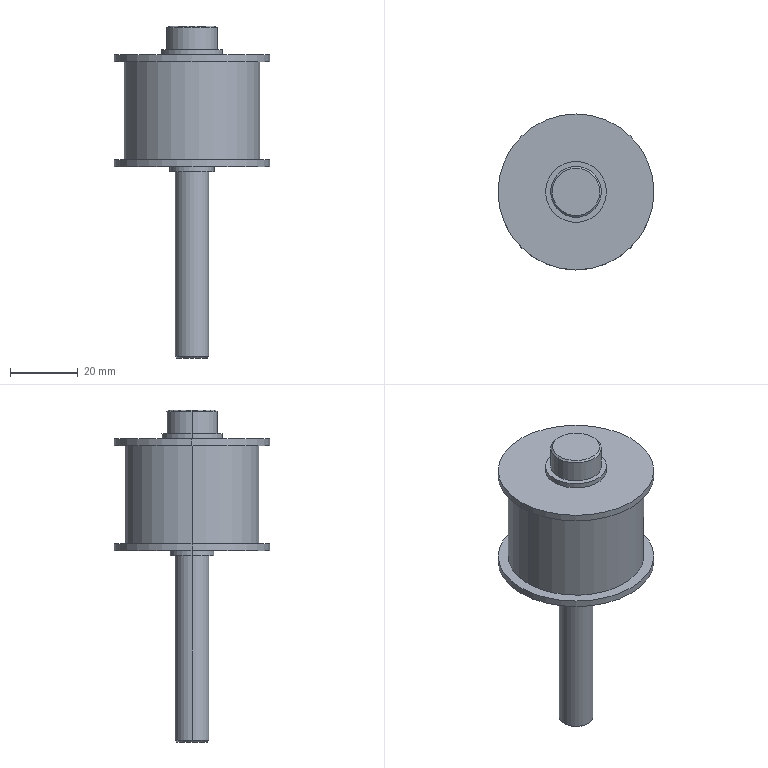Part | STEP file | (PA01.001.LX005) Drive Wheel A | 1 solid | 26 faces | box 46 x 46 x 98 mm | volume 49218 mm3 | cylinder 14 | plane 8 | cone 4 | commonest cylinder face diameters 46 x4 10 x2 13 x2 15 x2 18 x2 40 x2
STEP:
#1=CARTESIAN_POINT('',(0.,0.,0.));
#2=DIRECTION('',(0.,0.,1.));
#3=DIRECTION('',(1.,0.,0.));
#4=AXIS2_PLACEMENT_3D('',#1,#2,#3);
#5=CARTESIAN_POINT('',(7.,0.,25.));
#6=VERTEX_POINT('',#5);
#7=CARTESIAN_POINT('',(-7.,0.,25.));
#8=VERTEX_POINT('',#7);
#9=CARTESIAN_POINT('',(0.,0.,25.));
#10=DIRECTION('',(0.,0.,1.));
#11=DIRECTION('',(1.,0.,0.));
#12=AXIS2_PLACEMENT_3D('',#9,#10,#11);
#13=CIRCLE('',#12,7.);
#14=CARTESIAN_POINT('',(0.,0.,25.));
#15=DIRECTION('',(0.,0.,-1.));
#16=DIRECTION('',(-1.,0.,0.));
#17=AXIS2_PLACEMENT_3D('',#14,#15,#16);
#18=CONICAL_SURFACE('',#17,7.,0.7854);
#19=CARTESIAN_POINT('',(3.142,0.));
#20=DIRECTION('',(-1.,0.));
#21=VECTOR('',#20,1.);
#22=LINE('',#19,#21);
#23=(GEOMETRIC_REPRESENTATION_CONTEXT(2)PARAMETRIC_REPRESENTATION_CONTEXT()REPRESENTATION_CONTEXT('',''));
#24=DEFINITIONAL_REPRESENTATION('',(#22),#23);
#25=PCURVE('',#18,#24);
#26=CARTESIAN_POINT('',(0.,0.,25.));
#27=DIRECTION('',(0.,0.,1.));
#28=DIRECTION('',(1.,0.,0.));
#29=AXIS2_PLACEMENT_3D('',#26,#27,#28);
#30=PLANE('',#29);
#31=CARTESIAN_POINT('',(0.,0.));
#32=DIRECTION('',(1.,0.));
#33=AXIS2_PLACEMENT_2D('',#31,#32);
#34=CIRCLE('',#33,7.);
#35=(GEOMETRIC_REPRESENTATION_CONTEXT(2)PARAMETRIC_REPRESENTATION_CONTEXT()REPRESENTATION_CONTEXT('',''));
#36=DEFINITIONAL_REPRESENTATION('',(#34),#35);
#37=PCURVE('',#30,#36);
#38=SURFACE_CURVE('',#13,(#25,#37),.PCURVE_S1.);
#39=EDGE_CURVE('',#6,#8,#38,.T.);
#40=ORIENTED_EDGE('',*,*,#39,.F.);
#41=CARTESIAN_POINT('',(7.5,0.,24.5));
#42=VERTEX_POINT('',#41);
#43=CARTESIAN_POINT('',(7.,0.,25.));
#44=DIRECTION('',(0.7071,0.,-0.7071));
#45=VECTOR('',#44,1.);
#46=LINE('',#43,#45);
#47=CARTESIAN_POINT('',(3.142,0.));
#48=DIRECTION('',(0.,1.));
#49=VECTOR('',#48,1.);
#50=LINE('',#47,#49);
#51=(GEOMETRIC_REPRESENTATION_CONTEXT(2)PARAMETRIC_REPRESENTATION_CONTEXT()REPRESENTATION_CONTEXT('',''));
#52=DEFINITIONAL_REPRESENTATION('',(#50),#51);
#53=PCURVE('',#18,#52);
#54=CARTESIAN_POINT('',(0.,0.,25.));
#55=DIRECTION('',(0.,0.,-1.));
#56=DIRECTION('',(-1.,0.,0.));
#57=AXIS2_PLACEMENT_3D('',#54,#55,#56);
#58=CONICAL_SURFACE('',#57,7.,0.7854);
#59=CARTESIAN_POINT('',(3.142,0.));
#60=DIRECTION('',(0.,1.));
#61=VECTOR('',#60,1.);
#62=LINE('',#59,#61);
#63=(GEOMETRIC_REPRESENTATION_CONTEXT(2)PARAMETRIC_REPRESENTATION_CONTEXT()REPRESENTATION_CONTEXT('',''));
#64=DEFINITIONAL_REPRESENTATION('',(#62),#63);
#65=PCURVE('',#58,#64);
#66=SURFACE_CURVE('',#46,(#53,#65),.PCURVE_S1.);
#67=EDGE_CURVE('',#6,#42,#66,.T.);
#68=ORIENTED_EDGE('',*,*,#67,.T.);
#69=CARTESIAN_POINT('',(-7.5,0.,24.5));
#70=VERTEX_POINT('',#69);
#71=CARTESIAN_POINT('',(0.,0.,24.5));
#72=DIRECTION('',(0.,0.,-1.));
#73=DIRECTION('',(1.,0.,0.));
#74=AXIS2_PLACEMENT_3D('',#71,#72,#73);
#75=CIRCLE('',#74,7.5);
#76=CARTESIAN_POINT('',(-3.142,0.5));
#77=DIRECTION('',(1.,0.));
#78=VECTOR('',#77,1.);
#79=LINE('',#76,#78);
#80=(GEOMETRIC_REPRESENTATION_CONTEXT(2)PARAMETRIC_REPRESENTATION_CONTEXT()REPRESENTATION_CONTEXT('',''));
#81=DEFINITIONAL_REPRESENTATION('',(#79),#80);
#82=PCURVE('',#18,#81);
#83=CARTESIAN_POINT('',(0.,0.,25.));
#84=DIRECTION('',(0.,0.,-1.));
#85=DIRECTION('',(-1.,0.,0.));
#86=AXIS2_PLACEMENT_3D('',#83,#84,#85);
#87=CYLINDRICAL_SURFACE('',#86,7.5);
#88=CARTESIAN_POINT('',(-3.142,0.5));
#89=DIRECTION('',(1.,0.));
#90=VECTOR('',#89,1.);
#91=LINE('',#88,#90);
#92=(GEOMETRIC_REPRESENTATION_CONTEXT(2)PARAMETRIC_REPRESENTATION_CONTEXT()REPRESENTATION_CONTEXT('',''));
#93=DEFINITIONAL_REPRESENTATION('',(#91),#92);
#94=PCURVE('',#87,#93);
#95=SURFACE_CURVE('',#75,(#82,#94),.PCURVE_S1.);
#96=EDGE_CURVE('',#70,#42,#95,.T.);
#97=ORIENTED_EDGE('',*,*,#96,.F.);
#98=CARTESIAN_POINT('',(-7.,0.,25.));
#99=DIRECTION('',(-0.7071,0.,-0.7071));
#100=VECTOR('',#99,1.);
#101=LINE('',#98,#100);
#102=CARTESIAN_POINT('',(0.,0.));
#103=DIRECTION('',(0.,1.));
#104=VECTOR('',#103,1.);
#105=LINE('',#102,#104);
#106=(GEOMETRIC_REPRESENTATION_CONTEXT(2)PARAMETRIC_REPRESENTATION_CONTEXT()REPRESENTATION_CONTEXT('',''));
#107=DEFINITIONAL_REPRESENTATION('',(#105),#106);
#108=PCURVE('',#18,#107);
#109=CARTESIAN_POINT('',(6.283,0.));
#110=DIRECTION('',(0.,1.));
#111=VECTOR('',#110,1.);
#112=LINE('',#109,#111);
#113=(GEOMETRIC_REPRESENTATION_CONTEXT(2)PARAMETRIC_REPRESENTATION_CONTEXT()REPRESENTATION_CONTEXT('',''));
#114=DEFINITIONAL_REPRESENTATION('',(#112),#113);
#115=PCURVE('',#58,#114);
#116=SURFACE_CURVE('',#101,(#108,#115),.PCURVE_S1.);
#117=EDGE_CURVE('',#8,#70,#116,.T.);
#118=ORIENTED_EDGE('',*,*,#117,.F.);
#119=EDGE_LOOP('',(#40,#68,#97,#118));
#120=FACE_BOUND('',#119,.T.);
#121=ADVANCED_FACE('',(#120),#18,.T.);
#122=CARTESIAN_POINT('',(-4.5,0.,-73.));
#123=VERTEX_POINT('',#122);
#124=CARTESIAN_POINT('',(4.5,0.,-73.));
#125=VERTEX_POINT('',#124);
#126=CARTESIAN_POINT('',(0.,0.,-73.));
#127=DIRECTION('',(0.,0.,-1.));
#128=DIRECTION('',(-1.,0.,0.));
#129=AXIS2_PLACEMENT_3D('',#126,#127,#128);
#130=CIRCLE('',#129,4.5);
#131=CARTESIAN_POINT('',(0.,0.,-73.));
#132=DIRECTION('',(0.,0.,1.));
#133=DIRECTION('',(1.,0.,0.));
#134=AXIS2_PLACEMENT_3D('',#131,#132,#133);
#135=CONICAL_SURFACE('',#134,4.5,0.7854);
#136=CARTESIAN_POINT('',(3.142,0.));
#137=DIRECTION('',(-1.,0.));
#138=VECTOR('',#137,1.);
#139=LINE('',#136,#138);
#140=(GEOMETRIC_REPRESENTATION_CONTEXT(2)PARAMETRIC_REPRESENTATION_CONTEXT()REPRESENTATION_CONTEXT('',''));
#141=DEFINITIONAL_REPRESENTATION('',(#139),#140);
#142=PCURVE('',#135,#141);
#143=CARTESIAN_POINT('',(0.,0.,-73.));
#144=DIRECTION('',(0.,0.,-1.));
#145=DIRECTION('',(-1.,0.,0.));
#146=AXIS2_PLACEMENT_3D('',#143,#144,#145);
#147=PLANE('',#146);
#148=CARTESIAN_POINT('',(0.,0.));
#149=DIRECTION('',(1.,0.));
#150=AXIS2_PLACEMENT_2D('',#148,#149);
#151=CIRCLE('',#150,4.5);
#152=(GEOMETRIC_REPRESENTATION_CONTEXT(2)PARAMETRIC_REPRESENTATION_CONTEXT()REPRESENTATION_CONTEXT('',''));
#153=DEFINITIONAL_REPRESENTATION('',(#151),#152);
#154=PCURVE('',#147,#153);
#155=SURFACE_CURVE('',#130,(#142,#154),.PCURVE_S1.);
#156=EDGE_CURVE('',#123,#125,#155,.T.);
#157=ORIENTED_EDGE('',*,*,#156,.F.);
#158=CARTESIAN_POINT('',(-5.,0.,-72.5));
#159=VERTEX_POINT('',#158);
#160=CARTESIAN_POINT('',(-4.5,0.,-73.));
#161=DIRECTION('',(-0.7071,0.,0.7071));
#162=VECTOR('',#161,1.);
#163=LINE('',#160,#162);
#164=CARTESIAN_POINT('',(3.142,0.));
#165=DIRECTION('',(0.,1.));
#166=VECTOR('',#165,1.);
#167=LINE('',#164,#166);
#168=(GEOMETRIC_REPRESENTATION_CONTEXT(2)PARAMETRIC_REPRESENTATION_CONTEXT()REPRESENTATION_CONTEXT('',''));
#169=DEFINITIONAL_REPRESENTATION('',(#167),#168);
#170=PCURVE('',#135,#169);
#171=CARTESIAN_POINT('',(0.,0.,-73.));
#172=DIRECTION('',(0.,0.,1.));
#173=DIRECTION('',(1.,0.,0.));
#174=AXIS2_PLACEMENT_3D('',#171,#172,#173);
#175=CONICAL_SURFACE('',#174,4.5,0.7854);
#176=CARTESIAN_POINT('',(3.142,0.));
#177=DIRECTION('',(0.,1.));
#178=VECTOR('',#177,1.);
#179=LINE('',#176,#178);
#180=(GEOMETRIC_REPRESENTATION_CONTEXT(2)PARAMETRIC_REPRESENTATION_CONTEXT()REPRESENTATION_CONTEXT('',''));
#181=DEFINITIONAL_REPRESENTATION('',(#179),#180);
#182=PCURVE('',#175,#181);
#183=SURFACE_CURVE('',#163,(#170,#182),.PCURVE_S1.);
#184=EDGE_CURVE('',#123,#159,#183,.T.);
#185=ORIENTED_EDGE('',*,*,#184,.T.);
#186=CARTESIAN_POINT('',(5.,0.,-72.5));
#187=VERTEX_POINT('',#186);
#188=CARTESIAN_POINT('',(0.,0.,-72.5));
#189=DIRECTION('',(0.,0.,1.));
#190=DIRECTION('',(-1.,0.,0.));
#191=AXIS2_PLACEMENT_3D('',#188,#189,#190);
#192=CIRCLE('',#191,5.);
#193=CARTESIAN_POINT('',(-3.142,0.5));
#194=DIRECTION('',(1.,0.));
#195=VECTOR('',#194,1.);
#196=LINE('',#193,#195);
#197=(GEOMETRIC_REPRESENTATION_CONTEXT(2)PARAMETRIC_REPRESENTATION_CONTEXT()REPRESENTATION_CONTEXT('',''));
#198=DEFINITIONAL_REPRESENTATION('',(#196),#197);
#199=PCURVE('',#135,#198);
#200=CARTESIAN_POINT('',(0.,0.,-73.));
#201=DIRECTION('',(0.,0.,1.));
#202=DIRECTION('',(1.,0.,0.));
#203=AXIS2_PLACEMENT_3D('',#200,#201,#202);
#204=CYLINDRICAL_SURFACE('',#203,5.);
#205=CARTESIAN_POINT('',(-3.142,0.5));
#206=DIRECTION('',(1.,0.));
#207=VECTOR('',#206,1.);
#208=LINE('',#205,#207);
#209=(GEOMETRIC_REPRESENTATION_CONTEXT(2)PARAMETRIC_REPRESENTATION_CONTEXT()REPRESENTATION_CONTEXT('',''));
#210=DEFINITIONAL_REPRESENTATION('',(#208),#209);
#211=PCURVE('',#204,#210);
#212=SURFACE_CURVE('',#192,(#199,#211),.PCURVE_S1.);
#213=EDGE_CURVE('',#187,#159,#212,.T.);
#214=ORIENTED_EDGE('',*,*,#213,.F.);
#215=CARTESIAN_POINT('',(4.5,0.,-73.));
#216=DIRECTION('',(0.7071,0.,0.7071));
#217=VECTOR('',#216,1.);
#218=LINE('',#215,#217);
#219=CARTESIAN_POINT('',(0.,0.));
#220=DIRECTION('',(0.,1.));
#221=VECTOR('',#220,1.);
#222=LINE('',#219,#221);
#223=(GEOMETRIC_REPRESENTATION_CONTEXT(2)PARAMETRIC_REPRESENTATION_CONTEXT()REPRESENTATION_CONTEXT('',''));
#224=DEFINITIONAL_REPRESENTATION('',(#222),#223);
#225=PCURVE('',#135,#224);
#226=CARTESIAN_POINT('',(6.283,0.));
#227=DIRECTION('',(0.,1.));
#228=VECTOR('',#227,1.);
#229=LINE('',#226,#228);
#230=(GEOMETRIC_REPRESENTATION_CONTEXT(2)PARAMETRIC_REPRESENTATION_CONTEXT()REPRESENTATION_CONTEXT('',''));
#231=DEFINITIONAL_REPRESENTATION('',(#229),#230);
#232=PCURVE('',#175,#231);
#233=SURFACE_CURVE('',#218,(#225,#232),.PCURVE_S1.);
#234=EDGE_CURVE('',#125,#187,#233,.T.);
#235=ORIENTED_EDGE('',*,*,#234,.F.);
#236=EDGE_LOOP('',(#157,#185,#214,#235));
#237=FACE_BOUND('',#236,.T.);
#238=ADVANCED_FACE('',(#237),#135,.T.);
#239=ORIENTED_EDGE('',*,*,#213,.T.);
#240=CARTESIAN_POINT('',(-5.,0.,-18.));
#241=VERTEX_POINT('',#240);
#242=CARTESIAN_POINT('',(-5.,0.,-73.));
#243=DIRECTION('',(0.,0.,1.));
#244=VECTOR('',#243,1.);
#245=LINE('',#242,#244);
#246=CARTESIAN_POINT('',(3.142,0.));
#247=DIRECTION('',(0.,1.));
#248=VECTOR('',#247,1.);
#249=LINE('',#246,#248);
#250=(GEOMETRIC_REPRESENTATION_CONTEXT(2)PARAMETRIC_REPRESENTATION_CONTEXT()REPRESENTATION_CONTEXT('',''));
#251=DEFINITIONAL_REPRESENTATION('',(#249),#250);
#252=PCURVE('',#204,#251);
#253=CARTESIAN_POINT('',(0.,0.,-73.));
#254=DIRECTION('',(0.,0.,1.));
#255=DIRECTION('',(1.,0.,0.));
#256=AXIS2_PLACEMENT_3D('',#253,#254,#255);
#257=CYLINDRICAL_SURFACE('',#256,5.);
#258=CARTESIAN_POINT('',(3.142,0.));
#259=DIRECTION('',(0.,1.));
#260=VECTOR('',#259,1.);
#261=LINE('',#258,#260);
#262=(GEOMETRIC_REPRESENTATION_CONTEXT(2)PARAMETRIC_REPRESENTATION_CONTEXT()REPRESENTATION_CONTEXT('',''));
#263=DEFINITIONAL_REPRESENTATION('',(#261),#262);
#264=PCURVE('',#257,#263);
#265=SURFACE_CURVE('',#245,(#252,#264),.PCURVE_S1.);
#266=EDGE_CURVE('',#159,#241,#265,.T.);
#267=ORIENTED_EDGE('',*,*,#266,.T.);
#268=CARTESIAN_POINT('',(5.,0.,-18.));
#269=VERTEX_POINT('',#268);
#270=CARTESIAN_POINT('',(0.,0.,-18.));
#271=DIRECTION('',(0.,0.,-1.));
#272=DIRECTION('',(-1.,0.,0.));
#273=AXIS2_PLACEMENT_3D('',#270,#271,#272);
#274=CIRCLE('',#273,5.);
#275=CARTESIAN_POINT('',(3.142,55.));
#276=DIRECTION('',(-1.,0.));
#277=VECTOR('',#276,1.);
#278=LINE('',#275,#277);
#279=(GEOMETRIC_REPRESENTATION_CONTEXT(2)PARAMETRIC_REPRESENTATION_CONTEXT()REPRESENTATION_CONTEXT('',''));
#280=DEFINITIONAL_REPRESENTATION('',(#278),#279);
#281=PCURVE('',#204,#280);
#282=CARTESIAN_POINT('',(0.,0.,-18.));
#283=DIRECTION('',(0.,0.,-1.));
#284=DIRECTION('',(-1.,0.,0.));
#285=AXIS2_PLACEMENT_3D('',#282,#283,#284);
#286=PLANE('',#285);
#287=CARTESIAN_POINT('',(0.,0.));
#288=DIRECTION('',(1.,0.));
#289=AXIS2_PLACEMENT_2D('',#287,#288);
#290=CIRCLE('',#289,5.);
#291=(GEOMETRIC_REPRESENTATION_CONTEXT(2)PARAMETRIC_REPRESENTATION_CONTEXT()REPRESENTATION_CONTEXT('',''));
#292=DEFINITIONAL_REPRESENTATION('',(#290),#291);
#293=PCURVE('',#286,#292);
#294=SURFACE_CURVE('',#274,(#281,#293),.PCURVE_S1.);
#295=EDGE_CURVE('',#241,#269,#294,.T.);
#296=ORIENTED_EDGE('',*,*,#295,.T.);
#297=CARTESIAN_POINT('',(5.,0.,-73.));
#298=DIRECTION('',(0.,0.,1.));
#299=VECTOR('',#298,1.);
#300=LINE('',#297,#299);
#301=CARTESIAN_POINT('',(0.,0.));
#302=DIRECTION('',(0.,1.));
#303=VECTOR('',#302,1.);
#304=LINE('',#301,#303);
#305=(GEOMETRIC_REPRESENTATION_CONTEXT(2)PARAMETRIC_REPRESENTATION_CONTEXT()REPRESENTATION_CONTEXT('',''));
#306=DEFINITIONAL_REPRESENTATION('',(#304),#305);
#307=PCURVE('',#204,#306);
#308=CARTESIAN_POINT('',(6.283,0.));
#309=DIRECTION('',(0.,1.));
#310=VECTOR('',#309,1.);
#311=LINE('',#308,#310);
#312=(GEOMETRIC_REPRESENTATION_CONTEXT(2)PARAMETRIC_REPRESENTATION_CONTEXT()REPRESENTATION_CONTEXT('',''));
#313=DEFINITIONAL_REPRESENTATION('',(#311),#312);
#314=PCURVE('',#257,#313);
#315=SURFACE_CURVE('',#300,(#307,#314),.PCURVE_S1.);
#316=EDGE_CURVE('',#187,#269,#315,.T.);
#317=ORIENTED_EDGE('',*,*,#316,.F.);
#318=EDGE_LOOP('',(#239,#267,#296,#317));
#319=FACE_BOUND('',#318,.T.);
#320=ADVANCED_FACE('',(#319),#204,.T.);
#321=CARTESIAN_POINT('',(-6.5,0.,-18.));
#322=VERTEX_POINT('',#321);
#323=CARTESIAN_POINT('',(6.5,0.,-18.));
#324=VERTEX_POINT('',#323);
#325=CARTESIAN_POINT('',(0.,0.,-18.));
#326=DIRECTION('',(0.,0.,-1.));
#327=DIRECTION('',(-1.,0.,0.));
#328=AXIS2_PLACEMENT_3D('',#325,#326,#327);
#329=CIRCLE('',#328,6.5);
#330=CARTESIAN_POINT('',(0.,0.,-18.));
#331=DIRECTION('',(0.,0.,1.));
#332=DIRECTION('',(1.,0.,0.));
#333=AXIS2_PLACEMENT_3D('',#330,#331,#332);
#334=CYLINDRICAL_SURFACE('',#333,6.5);
#335=CARTESIAN_POINT('',(3.142,0.));
#336=DIRECTION('',(-1.,0.));
#337=VECTOR('',#336,1.);
#338=LINE('',#335,#337);
#339=(GEOMETRIC_REPRESENTATION_CONTEXT(2)PARAMETRIC_REPRESENTATION_CONTEXT()REPRESENTATION_CONTEXT('',''));
#340=DEFINITIONAL_REPRESENTATION('',(#338),#339);
#341=PCURVE('',#334,#340);
#342=CARTESIAN_POINT('',(0.,0.));
#343=DIRECTION('',(1.,0.));
#344=AXIS2_PLACEMENT_2D('',#342,#343);
#345=CIRCLE('',#344,6.5);
#346=(GEOMETRIC_REPRESENTATION_CONTEXT(2)PARAMETRIC_REPRESENTATION_CONTEXT()REPRESENTATION_CONTEXT('',''));
#347=DEFINITIONAL_REPRESENTATION('',(#345),#346);
#348=PCURVE('',#286,#347);
#349=SURFACE_CURVE('',#329,(#341,#348),.PCURVE_S1.);
#350=EDGE_CURVE('',#322,#324,#349,.T.);
#351=ORIENTED_EDGE('',*,*,#350,.F.);
#352=CARTESIAN_POINT('',(-6.5,0.,-16.5));
#353=VERTEX_POINT('',#352);
#354=CARTESIAN_POINT('',(-6.5,0.,-18.));
#355=DIRECTION('',(0.,0.,1.));
#356=VECTOR('',#355,1.);
#357=LINE('',#354,#356);
#358=CARTESIAN_POINT('',(3.142,0.));
#359=DIRECTION('',(0.,1.));
#360=VECTOR('',#359,1.);
#361=LINE('',#358,#360);
#362=(GEOMETRIC_REPRESENTATION_CONTEXT(2)PARAMETRIC_REPRESENTATION_CONTEXT()REPRESENTATION_CONTEXT('',''));
#363=DEFINITIONAL_REPRESENTATION('',(#361),#362);
#364=PCURVE('',#334,#363);
#365=CARTESIAN_POINT('',(0.,0.,-18.));
#366=DIRECTION('',(0.,0.,1.));
#367=DIRECTION('',(1.,0.,0.));
#368=AXIS2_PLACEMENT_3D('',#365,#366,#367);
#369=CYLINDRICAL_SURFACE('',#368,6.5);
#370=CARTESIAN_POINT('',(3.142,0.));
#371=DIRECTION('',(0.,1.));
#372=VECTOR('',#371,1.);
#373=LINE('',#370,#372);
#374=(GEOMETRIC_REPRESENTATION_CONTEXT(2)PARAMETRIC_REPRESENTATION_CONTEXT()REPRESENTATION_CONTEXT('',''));
#375=DEFINITIONAL_REPRESENTATION('',(#373),#374);
#376=PCURVE('',#369,#375);
#377=SURFACE_CURVE('',#357,(#364,#376),.PCURVE_S1.);
#378=EDGE_CURVE('',#322,#353,#377,.T.);
#379=ORIENTED_EDGE('',*,*,#378,.T.);
#380=CARTESIAN_POINT('',(6.5,0.,-16.5));
#381=VERTEX_POINT('',#380);
#382=CARTESIAN_POINT('',(0.,0.,-16.5));
#383=DIRECTION('',(0.,0.,-1.));
#384=DIRECTION('',(1.,0.,0.));
#385=AXIS2_PLACEMENT_3D('',#382,#383,#384);
#386=CIRCLE('',#385,6.5);
#387=CARTESIAN_POINT('',(6.283,1.5));
#388=DIRECTION('',(-1.,0.));
#389=VECTOR('',#388,1.);
#390=LINE('',#387,#389);
#391=(GEOMETRIC_REPRESENTATION_CONTEXT(2)PARAMETRIC_REPRESENTATION_CONTEXT()REPRESENTATION_CONTEXT('',''));
#392=DEFINITIONAL_REPRESENTATION('',(#390),#391);
#393=PCURVE('',#334,#392);
#394=CARTESIAN_POINT('',(0.,0.,-16.5));
#395=DIRECTION('',(0.,0.,1.));
#396=DIRECTION('',(1.,0.,0.));
#397=AXIS2_PLACEMENT_3D('',#394,#395,#396);
#398=PLANE('',#397);
#399=CARTESIAN_POINT('',(6.5,0.));
#400=CARTESIAN_POINT('',(6.5,-11.258));
#401=CARTESIAN_POINT('',(-3.25,-5.629));
#402=CARTESIAN_POINT('',(-13.,0.));
#403=CARTESIAN_POINT('',(-3.25,5.629));
#404=CARTESIAN_POINT('',(6.5,11.258));
#405=CARTESIAN_POINT('',(6.5,0.));
#406=(BOUNDED_CURVE()B_SPLINE_CURVE(2,(#399,#400,#401,#402,#403,#404,#405),.UNSPECIFIED.,.T.,.F.)B_SPLINE_CURVE_WITH_KNOTS((1,2,2,2,2,1),(-2.094,0.,2.094,4.189,6.283,8.378),.UNSPECIFIED.)CURVE()GEOMETRIC_REPRESENTATION_ITEM()RATIONAL_B_SPLINE_CURVE((1.,0.5,1.,0.5,1.,0.5,1.))REPRESENTATION_ITEM(''));
#407=(GEOMETRIC_REPRESENTATION_CONTEXT(2)PARAMETRIC_REPRESENTATION_CONTEXT()REPRESENTATION_CONTEXT('',''));
#408=DEFINITIONAL_REPRESENTATION('',(#406),#407);
#409=PCURVE('',#398,#408);
#410=SURFACE_CURVE('',#386,(#393,#409),.PCURVE_S1.);
#411=EDGE_CURVE('',#353,#381,#410,.T.);
#412=ORIENTED_EDGE('',*,*,#411,.T.);
#413=CARTESIAN_POINT('',(6.5,0.,-18.));
#414=DIRECTION('',(0.,0.,1.));
#415=VECTOR('',#414,1.);
#416=LINE('',#413,#415);
#417=CARTESIAN_POINT('',(0.,0.));
#418=DIRECTION('',(0.,1.));
#419=VECTOR('',#418,1.);
#420=LINE('',#417,#419);
#421=(GEOMETRIC_REPRESENTATION_CONTEXT(2)PARAMETRIC_REPRESENTATION_CONTEXT()REPRESENTATION_CONTEXT('',''));
#422=DEFINITIONAL_REPRESENTATION('',(#420),#421);
#423=PCURVE('',#334,#422);
#424=CARTESIAN_POINT('',(6.283,0.));
#425=DIRECTION('',(0.,1.));
#426=VECTOR('',#425,1.);
#427=LINE('',#424,#426);
#428=(GEOMETRIC_REPRESENTATION_CONTEXT(2)PARAMETRIC_REPRESENTATION_CONTEXT()REPRESENTATION_CONTEXT('',''));
#429=DEFINITIONAL_REPRESENTATION('',(#427),#428);
#430=PCURVE('',#369,#429);
#431=SURFACE_CURVE('',#416,(#423,#430),.PCURVE_S1.);
#432=EDGE_CURVE('',#324,#381,#431,.T.);
#433=ORIENTED_EDGE('',*,*,#432,.F.);
#434=EDGE_LOOP('',(#351,#379,#412,#433));
#435=FACE_BOUND('',#434,.T.);
#436=ADVANCED_FACE('',(#435),#334,.T.);
#437=CARTESIAN_POINT('',(-23.,0.,-14.5));
#438=VERTEX_POINT('',#437);
#439=CARTESIAN_POINT('',(23.,0.,-14.5));
#440=VERTEX_POINT('',#439);
#441=CARTESIAN_POINT('',(0.,0.,-14.5));
#442=DIRECTION('',(0.,0.,-1.));
#443=DIRECTION('',(-1.,0.,0.));
#444=AXIS2_PLACEMENT_3D('',#441,#442,#443);
#445=CIRCLE('',#444,23.);
#446=CARTESIAN_POINT('',(0.,0.,-14.5));
#447=DIRECTION('',(0.,0.,-1.));
#448=DIRECTION('',(-1.,0.,0.));
#449=AXIS2_PLACEMENT_3D('',#446,#447,#448);
#450=CYLINDRICAL_SURFACE('',#449,23.);
#451=CARTESIAN_POINT('',(0.,0.));
#452=DIRECTION('',(1.,0.));
#453=VECTOR('',#452,1.);
#454=LINE('',#451,#453);
#455=(GEOMETRIC_REPRESENTATION_CONTEXT(2)PARAMETRIC_REPRESENTATION_CONTEXT()REPRESENTATION_CONTEXT('',''));
#456=DEFINITIONAL_REPRESENTATION('',(#454),#455);
#457=PCURVE('',#450,#456);
#458=CARTESIAN_POINT('',(0.,0.,-14.5));
#459=DIRECTION('',(0.,0.,-1.));
#460=DIRECTION('',(-1.,0.,0.));
#461=AXIS2_PLACEMENT_3D('',#458,#459,#460);
#462=PLANE('',#461);
#463=CARTESIAN_POINT('',(0.,0.));
#464=DIRECTION('',(1.,0.));
#465=AXIS2_PLACEMENT_2D('',#463,#464);
#466=CIRCLE('',#465,23.);
#467=(GEOMETRIC_REPRESENTATION_CONTEXT(2)PARAMETRIC_REPRESENTATION_CONTEXT()REPRESENTATION_CONTEXT('',''));
#468=DEFINITIONAL_REPRESENTATION('',(#466),#467);
#469=PCURVE('',#462,#468);
#470=SURFACE_CURVE('',#445,(#457,#469),.PCURVE_S1.);
#471=EDGE_CURVE('',#438,#440,#470,.T.);
#472=ORIENTED_EDGE('',*,*,#471,.T.);
#473=CARTESIAN_POINT('',(23.,0.,-16.5));
#474=VERTEX_POINT('',#473);
#475=CARTESIAN_POINT('',(23.,0.,-14.5));
#476=DIRECTION('',(0.,0.,-1.));
#477=VECTOR('',#476,1.);
#478=LINE('',#475,#477);
#479=CARTESIAN_POINT('',(3.142,0.));
#480=DIRECTION('',(0.,1.));
#481=VECTOR('',#480,1.);
#482=LINE('',#479,#481);
#483=(GEOMETRIC_REPRESENTATION_CONTEXT(2)PARAMETRIC_REPRESENTATION_CONTEXT()REPRESENTATION_CONTEXT('',''));
#484=DEFINITIONAL_REPRESENTATION('',(#482),#483);
#485=PCURVE('',#450,#484);
#486=CARTESIAN_POINT('',(0.,0.,-14.5));
#487=DIRECTION('',(0.,0.,-1.));
#488=DIRECTION('',(-1.,0.,0.));
#489=AXIS2_PLACEMENT_3D('',#486,#487,#488);
#490=CYLINDRICAL_SURFACE('',#489,23.);
#491=CARTESIAN_POINT('',(3.142,0.));
#492=DIRECTION('',(0.,1.));
#493=VECTOR('',#492,1.);
#494=LINE('',#491,#493);
#495=(GEOMETRIC_REPRESENTATION_CONTEXT(2)PARAMETRIC_REPRESENTATION_CONTEXT()REPRESENTATION_CONTEXT('',''));
#496=DEFINITIONAL_REPRESENTATION('',(#494),#495);
#497=PCURVE('',#490,#496);
#498=SURFACE_CURVE('',#478,(#485,#497),.PCURVE_S1.);
#499=EDGE_CURVE('',#440,#474,#498,.T.);
#500=ORIENTED_EDGE('',*,*,#499,.T.);
#501=CARTESIAN_POINT('',(-23.,0.,-16.5));
#502=VERTEX_POINT('',#501);
#503=CARTESIAN_POINT('',(0.,0.,-16.5));
#504=DIRECTION('',(0.,0.,-1.));
#505=DIRECTION('',(-1.,0.,0.));
#506=AXIS2_PLACEMENT_3D('',#503,#504,#505);
#507=CIRCLE('',#506,23.);
#508=CARTESIAN_POINT('',(0.,2.));
#509=DIRECTION('',(1.,0.));
#510=VECTOR('',#509,1.);
#511=LINE('',#508,#510);
#512=(GEOMETRIC_REPRESENTATION_CONTEXT(2)PARAMETRIC_REPRESENTATION_CONTEXT()REPRESENTATION_CONTEXT('',''));
#513=DEFINITIONAL_REPRESENTATION('',(#511),#512);
#514=PCURVE('',#450,#513);
#515=CARTESIAN_POINT('',(-23.,0.));
#516=CARTESIAN_POINT('',(-23.,39.837));
#517=CARTESIAN_POINT('',(11.5,19.919));
#518=CARTESIAN_POINT('',(46.,0.));
#519=CARTESIAN_POINT('',(11.5,-19.919));
#520=CARTESIAN_POINT('',(-23.,-39.837));
#521=CARTESIAN_POINT('',(-23.,0.));
#522=(BOUNDED_CURVE()B_SPLINE_CURVE(2,(#515,#516,#517,#518,#519,#520,#521),.UNSPECIFIED.,.T.,.F.)B_SPLINE_CURVE_WITH_KNOTS((1,2,2,2,2,1),(-2.094,0.,2.094,4.189,6.283,8.378),.UNSPECIFIED.)CURVE()GEOMETRIC_REPRESENTATION_ITEM()RATIONAL_B_SPLINE_CURVE((1.,0.5,1.,0.5,1.,0.5,1.))REPRESENTATION_ITEM(''));
#523=(GEOMETRIC_REPRESENTATION_CONTEXT(2)PARAMETRIC_REPRESENTATION_CONTEXT()REPRESENTATION_CONTEXT('',''));
#524=DEFINITIONAL_REPRESENTATION('',(#522),#523);
#525=PCURVE('',#398,#524);
#526=SURFACE_CURVE('',#507,(#514,#525),.PCURVE_S1.);
#527=EDGE_CURVE('',#502,#474,#526,.T.);
#528=ORIENTED_EDGE('',*,*,#527,.F.);
#529=CARTESIAN_POINT('',(-23.,0.,-14.5));
#530=DIRECTION('',(0.,0.,-1.));
#531=VECTOR('',#530,1.);
#532=LINE('',#529,#531);
#533=CARTESIAN_POINT('',(0.,0.));
#534=DIRECTION('',(0.,1.));
#535=VECTOR('',#534,1.);
#536=LINE('',#533,#535);
#537=(GEOMETRIC_REPRESENTATION_CONTEXT(2)PARAMETRIC_REPRESENTATION_CONTEXT()REPRESENTATION_CONTEXT('',''));
#538=DEFINITIONAL_REPRESENTATION('',(#536),#537);
#539=PCURVE('',#450,#538);
#540=CARTESIAN_POINT('',(6.283,0.));
#541=DIRECTION('',(0.,1.));
#542=VECTOR('',#541,1.);
#543=LINE('',#540,#542);
#544=(GEOMETRIC_REPRESENTATION_CONTEXT(2)PARAMETRIC_REPRESENTATION_CONTEXT()REPRESENTATION_CONTEXT('',''));
#545=DEFINITIONAL_REPRESENTATION('',(#543),#544);
#546=PCURVE('',#490,#545);
#547=SURFACE_CURVE('',#532,(#539,#546),.PCURVE_S1.);
#548=EDGE_CURVE('',#438,#502,#547,.T.);
#549=ORIENTED_EDGE('',*,*,#548,.F.);
#550=EDGE_LOOP('',(#472,#500,#528,#549));
#551=FACE_BOUND('',#550,.T.);
#552=ADVANCED_FACE('',(#551),#450,.T.);
#553=CARTESIAN_POINT('',(23.,0.,14.5));
#554=VERTEX_POINT('',#553);
#555=CARTESIAN_POINT('',(-23.,0.,14.5));
#556=VERTEX_POINT('',#555);
#557=CARTESIAN_POINT('',(0.,0.,14.5));
#558=DIRECTION('',(0.,0.,1.));
#559=DIRECTION('',(1.,0.,0.));
#560=AXIS2_PLACEMENT_3D('',#557,#558,#559);
#561=CIRCLE('',#560,23.);
#562=CARTESIAN_POINT('',(0.,0.,14.5));
#563=DIRECTION('',(0.,0.,1.));
#564=DIRECTION('',(1.,0.,0.));
#565=AXIS2_PLACEMENT_3D('',#562,#563,#564);
#566=CYLINDRICAL_SURFACE('',#565,23.);
#567=CARTESIAN_POINT('',(0.,0.));
#568=DIRECTION('',(1.,0.));
#569=VECTOR('',#568,1.);
#570=LINE('',#567,#569);
#571=(GEOMETRIC_REPRESENTATION_CONTEXT(2)PARAMETRIC_REPRESENTATION_CONTEXT()REPRESENTATION_CONTEXT('',''));
#572=DEFINITIONAL_REPRESENTATION('',(#570),#571);
#573=PCURVE('',#566,#572);
#574=CARTESIAN_POINT('',(0.,0.,14.5));
#575=DIRECTION('',(0.,0.,1.));
#576=DIRECTION('',(1.,0.,0.));
#577=AXIS2_PLACEMENT_3D('',#574,#575,#576);
#578=PLANE('',#577);
#579=CARTESIAN_POINT('',(0.,0.));
#580=DIRECTION('',(1.,0.));
#581=AXIS2_PLACEMENT_2D('',#579,#580);
#582=CIRCLE('',#581,23.);
#583=(GEOMETRIC_REPRESENTATION_CONTEXT(2)PARAMETRIC_REPRESENTATION_CONTEXT()REPRESENTATION_CONTEXT('',''));
#584=DEFINITIONAL_REPRESENTATION('',(#582),#583);
#585=PCURVE('',#578,#584);
#586=SURFACE_CURVE('',#561,(#573,#585),.PCURVE_S1.);
#587=EDGE_CURVE('',#554,#556,#586,.T.);
#588=ORIENTED_EDGE('',*,*,#587,.T.);
#589=CARTESIAN_POINT('',(-23.,0.,16.5));
#590=VERTEX_POINT('',#589);
#591=CARTESIAN_POINT('',(-23.,0.,14.5));
#592=DIRECTION('',(0.,0.,1.));
#593=VECTOR('',#592,1.);
#594=LINE('',#591,#593);
#595=CARTESIAN_POINT('',(3.142,0.));
#596=DIRECTION('',(0.,1.));
#597=VECTOR('',#596,1.);
#598=LINE('',#595,#597);
#599=(GEOMETRIC_REPRESENTATION_CONTEXT(2)PARAMETRIC_REPRESENTATION_CONTEXT()REPRESENTATION_CONTEXT('',''));
#600=DEFINITIONAL_REPRESENTATION('',(#598),#599);
#601=PCURVE('',#566,#600);
#602=CARTESIAN_POINT('',(0.,0.,14.5));
#603=DIRECTION('',(0.,0.,1.));
#604=DIRECTION('',(1.,0.,0.));
#605=AXIS2_PLACEMENT_3D('',#602,#603,#604);
#606=CYLINDRICAL_SURFACE('',#605,23.);
#607=CARTESIAN_POINT('',(3.142,0.));
#608=DIRECTION('',(0.,1.));
#609=VECTOR('',#608,1.);
#610=LINE('',#607,#609);
#611=(GEOMETRIC_REPRESENTATION_CONTEXT(2)PARAMETRIC_REPRESENTATION_CONTEXT()REPRESENTATION_CONTEXT('',''));
#612=DEFINITIONAL_REPRESENTATION('',(#610),#611);
#613=PCURVE('',#606,#612);
#614=SURFACE_CURVE('',#594,(#601,#613),.PCURVE_S1.);
#615=EDGE_CURVE('',#556,#590,#614,.T.);
#616=ORIENTED_EDGE('',*,*,#615,.T.);
#617=CARTESIAN_POINT('',(23.,0.,16.5));
#618=VERTEX_POINT('',#617);
#619=CARTESIAN_POINT('',(0.,0.,16.5));
#620=DIRECTION('',(0.,0.,1.));
#621=DIRECTION('',(1.,0.,0.));
#622=AXIS2_PLACEMENT_3D('',#619,#620,#621);
#623=CIRCLE('',#622,23.);
#624=CARTESIAN_POINT('',(0.,2.));
#625=DIRECTION('',(1.,0.));
#626=VECTOR('',#625,1.);
#627=LINE('',#624,#626);
#628=(GEOMETRIC_REPRESENTATION_CONTEXT(2)PARAMETRIC_REPRESENTATION_CONTEXT()REPRESENTATION_CONTEXT('',''));
#629=DEFINITIONAL_REPRESENTATION('',(#627),#628);
#630=PCURVE('',#566,#629);
#631=CARTESIAN_POINT('',(0.,0.,16.5));
#632=DIRECTION('',(0.,0.,1.));
#633=DIRECTION('',(1.,0.,0.));
#634=AXIS2_PLACEMENT_3D('',#631,#632,#633);
#635=PLANE('',#634);
#636=CARTESIAN_POINT('',(0.,0.));
#637=DIRECTION('',(1.,0.));
#638=AXIS2_PLACEMENT_2D('',#636,#637);
#639=CIRCLE('',#638,23.);
#640=(GEOMETRIC_REPRESENTATION_CONTEXT(2)PARAMETRIC_REPRESENTATION_CONTEXT()REPRESENTATION_CONTEXT('',''));
#641=DEFINITIONAL_REPRESENTATION('',(#639),#640);
#642=PCURVE('',#635,#641);
#643=SURFACE_CURVE('',#623,(#630,#642),.PCURVE_S1.);
#644=EDGE_CURVE('',#618,#590,#643,.T.);
#645=ORIENTED_EDGE('',*,*,#644,.F.);
#646=CARTESIAN_POINT('',(23.,0.,14.5));
#647=DIRECTION('',(0.,0.,1.));
#648=VECTOR('',#647,1.);
#649=LINE('',#646,#648);
#650=CARTESIAN_POINT('',(0.,0.));
#651=DIRECTION('',(0.,1.));
#652=VECTOR('',#651,1.);
#653=LINE('',#650,#652);
#654=(GEOMETRIC_REPRESENTATION_CONTEXT(2)PARAMETRIC_REPRESENTATION_CONTEXT()REPRESENTATION_CONTEXT('',''));
#655=DEFINITIONAL_REPRESENTATION('',(#653),#654);
#656=PCURVE('',#566,#655);
#657=CARTESIAN_POINT('',(6.283,0.));
#658=DIRECTION('',(0.,1.));
#659=VECTOR('',#658,1.);
#660=LINE('',#657,#659);
#661=(GEOMETRIC_REPRESENTATION_CONTEXT(2)PARAMETRIC_REPRESENTATION_CONTEXT()REPRESENTATION_CONTEXT('',''));
#662=DEFINITIONAL_REPRESENTATION('',(#660),#661);
#663=PCURVE('',#606,#662);
#664=SURFACE_CURVE('',#649,(#656,#663),.PCURVE_S1.);
#665=EDGE_CURVE('',#554,#618,#664,.T.);
#666=ORIENTED_EDGE('',*,*,#665,.F.);
#667=EDGE_LOOP('',(#588,#616,#645,#666));
#668=FACE_BOUND('',#667,.T.);
#669=ADVANCED_FACE('',(#668),#566,.T.);
#670=ORIENTED_EDGE('',*,*,#96,.T.);
#671=CARTESIAN_POINT('',(7.5,0.,18.));
#672=VERTEX_POINT('',#671);
#673=CARTESIAN_POINT('',(7.5,0.,25.));
#674=DIRECTION('',(0.,0.,-1.));
#675=VECTOR('',#674,1.);
#676=LINE('',#673,#675);
#677=CARTESIAN_POINT('',(3.142,0.));
#678=DIRECTION('',(0.,1.));
#679=VECTOR('',#678,1.);
#680=LINE('',#677,#679);
#681=(GEOMETRIC_REPRESENTATION_CONTEXT(2)PARAMETRIC_REPRESENTATION_CONTEXT()REPRESENTATION_CONTEXT('',''));
#682=DEFINITIONAL_REPRESENTATION('',(#680),#681);
#683=PCURVE('',#87,#682);
#684=CARTESIAN_POINT('',(0.,0.,25.));
#685=DIRECTION('',(0.,0.,-1.));
#686=DIRECTION('',(-1.,0.,0.));
#687=AXIS2_PLACEMENT_3D('',#684,#685,#686);
#688=CYLINDRICAL_SURFACE('',#687,7.5);
#689=CARTESIAN_POINT('',(3.142,0.));
#690=DIRECTION('',(0.,1.));
#691=VECTOR('',#690,1.);
#692=LINE('',#689,#691);
#693=(GEOMETRIC_REPRESENTATION_CONTEXT(2)PARAMETRIC_REPRESENTATION_CONTEXT()REPRESENTATION_CONTEXT('',''));
#694=DEFINITIONAL_REPRESENTATION('',(#692),#693);
#695=PCURVE('',#688,#694);
#696=SURFACE_CURVE('',#676,(#683,#695),.PCURVE_S1.);
#697=EDGE_CURVE('',#42,#672,#696,.T.);
#698=ORIENTED_EDGE('',*,*,#697,.T.);
#699=CARTESIAN_POINT('',(-7.5,0.,18.));
#700=VERTEX_POINT('',#699);
#701=CARTESIAN_POINT('',(0.,0.,18.));
#702=DIRECTION('',(0.,0.,1.));
#703=DIRECTION('',(1.,0.,0.));
#704=AXIS2_PLACEMENT_3D('',#701,#702,#703);
#705=CIRCLE('',#704,7.5);
#706=CARTESIAN_POINT('',(3.142,7.));
#707=DIRECTION('',(-1.,0.));
#708=VECTOR('',#707,1.);
#709=LINE('',#706,#708);
#710=(GEOMETRIC_REPRESENTATION_CONTEXT(2)PARAMETRIC_REPRESENTATION_CONTEXT()REPRESENTATION_CONTEXT('',''));
#711=DEFINITIONAL_REPRESENTATION('',(#709),#710);
#712=PCURVE('',#87,#711);
#713=CARTESIAN_POINT('',(0.,0.,18.));
#714=DIRECTION('',(0.,0.,1.));
#715=DIRECTION('',(1.,0.,0.));
#716=AXIS2_PLACEMENT_3D('',#713,#714,#715);
#717=PLANE('',#716);
#718=CARTESIAN_POINT('',(0.,0.));
#719=DIRECTION('',(1.,0.));
#720=AXIS2_PLACEMENT_2D('',#718,#719);
#721=CIRCLE('',#720,7.5);
#722=(GEOMETRIC_REPRESENTATION_CONTEXT(2)PARAMETRIC_REPRESENTATION_CONTEXT()REPRESENTATION_CONTEXT('',''));
#723=DEFINITIONAL_REPRESENTATION('',(#721),#722);
#724=PCURVE('',#717,#723);
#725=SURFACE_CURVE('',#705,(#712,#724),.PCURVE_S1.);
#726=EDGE_CURVE('',#672,#700,#725,.T.);
#727=ORIENTED_EDGE('',*,*,#726,.T.);
#728=CARTESIAN_POINT('',(-7.5,0.,25.));
#729=DIRECTION('',(0.,0.,-1.));
#730=VECTOR('',#729,1.);
#731=LINE('',#728,#730);
#732=CARTESIAN_POINT('',(0.,0.));
#733=DIRECTION('',(0.,1.));
#734=VECTOR('',#733,1.);
#735=LINE('',#732,#734);
#736=(GEOMETRIC_REPRESENTATION_CONTEXT(2)PARAMETRIC_REPRESENTATION_CONTEXT()REPRESENTATION_CONTEXT('',''));
#737=DEFINITIONAL_REPRESENTATION('',(#735),#736);
#738=PCURVE('',#87,#737);
#739=CARTESIAN_POINT('',(6.283,0.));
#740=DIRECTION('',(0.,1.));
#741=VECTOR('',#740,1.);
#742=LINE('',#739,#741);
#743=(GEOMETRIC_REPRESENTATION_CONTEXT(2)PARAMETRIC_REPRESENTATION_CONTEXT()REPRESENTATION_CONTEXT('',''));
#744=DEFINITIONAL_REPRESENTATION('',(#742),#743);
#745=PCURVE('',#688,#744);
#746=SURFACE_CURVE('',#731,(#738,#745),.PCURVE_S1.);
#747=EDGE_CURVE('',#70,#700,#746,.T.);
#748=ORIENTED_EDGE('',*,*,#747,.F.);
#749=EDGE_LOOP('',(#670,#698,#727,#748));
#750=FACE_BOUND('',#749,.T.);
#751=ADVANCED_FACE('',(#750),#87,.T.);
#752=CARTESIAN_POINT('',(9.,0.,18.));
#753=VERTEX_POINT('',#752);
#754=CARTESIAN_POINT('',(-9.,0.,18.));
#755=VERTEX_POINT('',#754);
#756=CARTESIAN_POINT('',(0.,0.,18.));
#757=DIRECTION('',(0.,0.,1.));
#758=DIRECTION('',(1.,0.,0.));
#759=AXIS2_PLACEMENT_3D('',#756,#757,#758);
#760=CIRCLE('',#759,9.);
#761=CARTESIAN_POINT('',(0.,0.,18.));
#762=DIRECTION('',(0.,0.,-1.));
#763=DIRECTION('',(-1.,0.,0.));
#764=AXIS2_PLACEMENT_3D('',#761,#762,#763);
#765=CYLINDRICAL_SURFACE('',#764,9.);
#766=CARTESIAN_POINT('',(3.142,0.));
#767=DIRECTION('',(-1.,0.));
#768=VECTOR('',#767,1.);
#769=LINE('',#766,#768);
#770=(GEOMETRIC_REPRESENTATION_CONTEXT(2)PARAMETRIC_REPRESENTATION_CONTEXT()REPRESENTATION_CONTEXT('',''));
#771=DEFINITIONAL_REPRESENTATION('',(#769),#770);
#772=PCURVE('',#765,#771);
#773=CARTESIAN_POINT('',(0.,0.));
#774=DIRECTION('',(1.,0.));
#775=AXIS2_PLACEMENT_2D('',#773,#774);
#776=CIRCLE('',#775,9.);
#777=(GEOMETRIC_REPRESENTATION_CONTEXT(2)PARAMETRIC_REPRESENTATION_CONTEXT()REPRESENTATION_CONTEXT('',''));
#778=DEFINITIONAL_REPRESENTATION('',(#776),#777);
#779=PCURVE('',#717,#778);
#780=SURFACE_CURVE('',#760,(#772,#779),.PCURVE_S1.);
#781=EDGE_CURVE('',#753,#755,#780,.T.);
#782=ORIENTED_EDGE('',*,*,#781,.F.);
#783=CARTESIAN_POINT('',(9.,0.,16.5));
#784=VERTEX_POINT('',#783);
#785=CARTESIAN_POINT('',(9.,0.,18.));
#786=DIRECTION('',(0.,0.,-1.));
#787=VECTOR('',#786,1.);
#788=LINE('',#785,#787);
#789=CARTESIAN_POINT('',(3.142,0.));
#790=DIRECTION('',(0.,1.));
#791=VECTOR('',#790,1.);
#792=LINE('',#789,#791);
#793=(GEOMETRIC_REPRESENTATION_CONTEXT(2)PARAMETRIC_REPRESENTATION_CONTEXT()REPRESENTATION_CONTEXT('',''));
#794=DEFINITIONAL_REPRESENTATION('',(#792),#793);
#795=PCURVE('',#765,#794);
#796=CARTESIAN_POINT('',(0.,0.,18.));
#797=DIRECTION('',(0.,0.,-1.));
#798=DIRECTION('',(-1.,0.,0.));
#799=AXIS2_PLACEMENT_3D('',#796,#797,#798);
#800=CYLINDRICAL_SURFACE('',#799,9.);
#801=CARTESIAN_POINT('',(3.142,0.));
#802=DIRECTION('',(0.,1.));
#803=VECTOR('',#802,1.);
#804=LINE('',#801,#803);
#805=(GEOMETRIC_REPRESENTATION_CONTEXT(2)PARAMETRIC_REPRESENTATION_CONTEXT()REPRESENTATION_CONTEXT('',''));
#806=DEFINITIONAL_REPRESENTATION('',(#804),#805);
#807=PCURVE('',#800,#806);
#808=SURFACE_CURVE('',#788,(#795,#807),.PCURVE_S1.);
#809=EDGE_CURVE('',#753,#784,#808,.T.);
#810=ORIENTED_EDGE('',*,*,#809,.T.);
#811=CARTESIAN_POINT('',(-9.,0.,16.5));
#812=VERTEX_POINT('',#811);
#813=CARTESIAN_POINT('',(0.,0.,16.5));
#814=DIRECTION('',(0.,0.,1.));
#815=DIRECTION('',(1.,0.,0.));
#816=AXIS2_PLACEMENT_3D('',#813,#814,#815);
#817=CIRCLE('',#816,9.);
#818=CARTESIAN_POINT('',(3.142,1.5));
#819=DIRECTION('',(-1.,0.));
#820=VECTOR('',#819,1.);
#821=LINE('',#818,#820);
#822=(GEOMETRIC_REPRESENTATION_CONTEXT(2)PARAMETRIC_REPRESENTATION_CONTEXT()REPRESENTATION_CONTEXT('',''));
#823=DEFINITIONAL_REPRESENTATION('',(#821),#822);
#824=PCURVE('',#765,#823);
#825=CARTESIAN_POINT('',(0.,0.));
#826=DIRECTION('',(1.,0.));
#827=AXIS2_PLACEMENT_2D('',#825,#826);
#828=CIRCLE('',#827,9.);
#829=(GEOMETRIC_REPRESENTATION_CONTEXT(2)PARAMETRIC_REPRESENTATION_CONTEXT()REPRESENTATION_CONTEXT('',''));
#830=DEFINITIONAL_REPRESENTATION('',(#828),#829);
#831=PCURVE('',#635,#830);
#832=SURFACE_CURVE('',#817,(#824,#831),.PCURVE_S1.);
#833=EDGE_CURVE('',#784,#812,#832,.T.);
#834=ORIENTED_EDGE('',*,*,#833,.T.);
#835=CARTESIAN_POINT('',(-9.,0.,18.));
#836=DIRECTION('',(0.,0.,-1.));
#837=VECTOR('',#836,1.);
#838=LINE('',#835,#837);
#839=CARTESIAN_POINT('',(0.,0.));
#840=DIRECTION('',(0.,1.));
#841=VECTOR('',#840,1.);
#842=LINE('',#839,#841);
#843=(GEOMETRIC_REPRESENTATION_CONTEXT(2)PARAMETRIC_REPRESENTATION_CONTEXT()REPRESENTATION_CONTEXT('',''));
#844=DEFINITIONAL_REPRESENTATION('',(#842),#843);
#845=PCURVE('',#765,#844);
#846=CARTESIAN_POINT('',(6.283,0.));
#847=DIRECTION('',(0.,1.));
#848=VECTOR('',#847,1.);
#849=LINE('',#846,#848);
#850=(GEOMETRIC_REPRESENTATION_CONTEXT(2)PARAMETRIC_REPRESENTATION_CONTEXT()REPRESENTATION_CONTEXT('',''));
#851=DEFINITIONAL_REPRESENTATION('',(#849),#850);
#852=PCURVE('',#800,#851);
#853=SURFACE_CURVE('',#838,(#845,#852),.PCURVE_S1.);
#854=EDGE_CURVE('',#755,#812,#853,.T.);
#855=ORIENTED_EDGE('',*,*,#854,.F.);
#856=EDGE_LOOP('',(#782,#810,#834,#855));
#857=FACE_BOUND('',#856,.T.);
#858=ADVANCED_FACE('',(#857),#765,.T.);
#859=CARTESIAN_POINT('',(20.,0.,14.5));
#860=VERTEX_POINT('',#859);
#861=CARTESIAN_POINT('',(-20.,0.,14.5));
#862=VERTEX_POINT('',#861);
#863=CARTESIAN_POINT('',(0.,0.,14.5));
#864=DIRECTION('',(0.,0.,1.));
#865=DIRECTION('',(1.,0.,0.));
#866=AXIS2_PLACEMENT_3D('',#863,#864,#865);
#867=CIRCLE('',#866,20.);
#868=CARTESIAN_POINT('',(0.,0.,16.5));
#869=DIRECTION('',(0.,0.,-1.));
#870=DIRECTION('',(-1.,0.,0.));
#871=AXIS2_PLACEMENT_3D('',#868,#869,#870);
#872=CYLINDRICAL_SURFACE('',#871,20.);
#873=CARTESIAN_POINT('',(3.142,2.));
#874=DIRECTION('',(-1.,0.));
#875=VECTOR('',#874,1.);
#876=LINE('',#873,#875);
#877=(GEOMETRIC_REPRESENTATION_CONTEXT(2)PARAMETRIC_REPRESENTATION_CONTEXT()REPRESENTATION_CONTEXT('',''));
#878=DEFINITIONAL_REPRESENTATION('',(#876),#877);
#879=PCURVE('',#872,#878);
#880=CARTESIAN_POINT('',(0.,0.));
#881=DIRECTION('',(1.,0.));
#882=AXIS2_PLACEMENT_2D('',#880,#881);
#883=CIRCLE('',#882,20.);
#884=(GEOMETRIC_REPRESENTATION_CONTEXT(2)PARAMETRIC_REPRESENTATION_CONTEXT()REPRESENTATION_CONTEXT('',''));
#885=DEFINITIONAL_REPRESENTATION('',(#883),#884);
#886=PCURVE('',#578,#885);
#887=SURFACE_CURVE('',#867,(#879,#886),.PCURVE_S1.);
#888=EDGE_CURVE('',#860,#862,#887,.T.);
#889=ORIENTED_EDGE('',*,*,#888,.F.);
#890=CARTESIAN_POINT('',(20.,0.,-14.5));
#891=VERTEX_POINT('',#890);
#892=CARTESIAN_POINT('',(20.,0.,16.5));
#893=DIRECTION('',(0.,0.,-1.));
#894=VECTOR('',#893,1.);
#895=LINE('',#892,#894);
#896=CARTESIAN_POINT('',(3.142,0.));
#897=DIRECTION('',(0.,1.));
#898=VECTOR('',#897,1.);
#899=LINE('',#896,#898);
#900=(GEOMETRIC_REPRESENTATION_CONTEXT(2)PARAMETRIC_REPRESENTATION_CONTEXT()REPRESENTATION_CONTEXT('',''));
#901=DEFINITIONAL_REPRESENTATION('',(#899),#900);
#902=PCURVE('',#872,#901);
#903=CARTESIAN_POINT('',(0.,0.,16.5));
#904=DIRECTION('',(0.,0.,-1.));
#905=DIRECTION('',(-1.,0.,0.));
#906=AXIS2_PLACEMENT_3D('',#903,#904,#905);
#907=CYLINDRICAL_SURFACE('',#906,20.);
#908=CARTESIAN_POINT('',(3.142,0.));
#909=DIRECTION('',(0.,1.));
#910=VECTOR('',#909,1.);
#911=LINE('',#908,#910);
#912=(GEOMETRIC_REPRESENTATION_CONTEXT(2)PARAMETRIC_REPRESENTATION_CONTEXT()REPRESENTATION_CONTEXT('',''));
#913=DEFINITIONAL_REPRESENTATION('',(#911),#912);
#914=PCURVE('',#907,#913);
#915=SURFACE_CURVE('',#895,(#902,#914),.PCURVE_S1.);
#916=EDGE_CURVE('',#860,#891,#915,.T.);
#917=ORIENTED_EDGE('',*,*,#916,.T.);
#918=CARTESIAN_POINT('',(-20.,0.,-14.5));
#919=VERTEX_POINT('',#918);
#920=CARTESIAN_POINT('',(0.,0.,-14.5));
#921=DIRECTION('',(0.,0.,-1.));
#922=DIRECTION('',(-1.,0.,0.));
#923=AXIS2_PLACEMENT_3D('',#920,#921,#922);
#924=CIRCLE('',#923,20.);
#925=CARTESIAN_POINT('',(0.,31.));
#926=DIRECTION('',(1.,0.));
#927=VECTOR('',#926,1.);
#928=LINE('',#925,#927);
#929=(GEOMETRIC_REPRESENTATION_CONTEXT(2)PARAMETRIC_REPRESENTATION_CONTEXT()REPRESENTATION_CONTEXT('',''));
#930=DEFINITIONAL_REPRESENTATION('',(#928),#929);
#931=PCURVE('',#872,#930);
#932=CARTESIAN_POINT('',(0.,0.));
#933=DIRECTION('',(1.,0.));
#934=AXIS2_PLACEMENT_2D('',#932,#933);
#935=CIRCLE('',#934,20.);
#936=(GEOMETRIC_REPRESENTATION_CONTEXT(2)PARAMETRIC_REPRESENTATION_CONTEXT()REPRESENTATION_CONTEXT('',''));
#937=DEFINITIONAL_REPRESENTATION('',(#935),#936);
#938=PCURVE('',#462,#937);
#939=SURFACE_CURVE('',#924,(#931,#938),.PCURVE_S1.);
#940=EDGE_CURVE('',#919,#891,#939,.T.);
#941=ORIENTED_EDGE('',*,*,#940,.F.);
#942=CARTESIAN_POINT('',(-20.,0.,16.5));
#943=DIRECTION('',(0.,0.,-1.));
#944=VECTOR('',#943,1.);
#945=LINE('',#942,#944);
#946=CARTESIAN_POINT('',(0.,0.));
#947=DIRECTION('',(0.,1.));
#948=VECTOR('',#947,1.);
#949=LINE('',#946,#948);
#950=(GEOMETRIC_REPRESENTATION_CONTEXT(2)PARAMETRIC_REPRESENTATION_CONTEXT()REPRESENTATION_CONTEXT('',''));
#951=DEFINITIONAL_REPRESENTATION('',(#949),#950);
#952=PCURVE('',#872,#951);
#953=CARTESIAN_POINT('',(6.283,0.));
#954=DIRECTION('',(0.,1.));
#955=VECTOR('',#954,1.);
#956=LINE('',#953,#955);
#957=(GEOMETRIC_REPRESENTATION_CONTEXT(2)PARAMETRIC_REPRESENTATION_CONTEXT()REPRESENTATION_CONTEXT('',''));
#958=DEFINITIONAL_REPRESENTATION('',(#956),#957);
#959=PCURVE('',#907,#958);
#960=SURFACE_CURVE('',#945,(#952,#959),.PCURVE_S1.);
#961=EDGE_CURVE('',#862,#919,#960,.T.);
#962=ORIENTED_EDGE('',*,*,#961,.F.);
#963=EDGE_LOOP('',(#889,#917,#941,#962));
#964=FACE_BOUND('',#963,.T.);
#965=ADVANCED_FACE('',(#964),#872,.T.);
#966=CARTESIAN_POINT('',(0.,0.,-18.));
#967=DIRECTION('',(0.,0.,-1.));
#968=DIRECTION('',(-1.,0.,0.));
#969=AXIS2_PLACEMENT_3D('',#966,#967,#968);
#970=CIRCLE('',#969,6.5);
#971=CARTESIAN_POINT('',(0.,0.));
#972=DIRECTION('',(1.,0.));
#973=AXIS2_PLACEMENT_2D('',#971,#972);
#974=CIRCLE('',#973,6.5);
#975=(GEOMETRIC_REPRESENTATION_CONTEXT(2)PARAMETRIC_REPRESENTATION_CONTEXT()REPRESENTATION_CONTEXT('',''));
#976=DEFINITIONAL_REPRESENTATION('',(#974),#975);
#977=PCURVE('',#286,#976);
#978=CARTESIAN_POINT('',(9.425,0.));
#979=DIRECTION('',(-1.,0.));
#980=VECTOR('',#979,1.);
#981=LINE('',#978,#980);
#982=(GEOMETRIC_REPRESENTATION_CONTEXT(2)PARAMETRIC_REPRESENTATION_CONTEXT()REPRESENTATION_CONTEXT('',''));
#983=DEFINITIONAL_REPRESENTATION('',(#981),#982);
#984=PCURVE('',#369,#983);
#985=SURFACE_CURVE('',#970,(#977,#984),.PCURVE_S1.);
#986=EDGE_CURVE('',#324,#322,#985,.T.);
#987=ORIENTED_EDGE('',*,*,#986,.T.);
#988=ORIENTED_EDGE('',*,*,#350,.T.);
#989=EDGE_LOOP('',(#987,#988));
#990=FACE_BOUND('',#989,.T.);
#991=CARTESIAN_POINT('',(0.,0.,-18.));
#992=DIRECTION('',(0.,0.,-1.));
#993=DIRECTION('',(-1.,0.,0.));
#994=AXIS2_PLACEMENT_3D('',#991,#992,#993);
#995=CIRCLE('',#994,5.);
#996=CARTESIAN_POINT('',(0.,0.));
#997=DIRECTION('',(1.,0.));
#998=AXIS2_PLACEMENT_2D('',#996,#997);
#999=CIRCLE('',#998,5.);
#1000=(GEOMETRIC_REPRESENTATION_CONTEXT(2)PARAMETRIC_REPRESENTATION_CONTEXT()REPRESENTATION_CONTEXT('',''));
#1001=DEFINITIONAL_REPRESENTATION('',(#999),#1000);
#1002=PCURVE('',#286,#1001);
#1003=CARTESIAN_POINT('',(9.425,55.));
#1004=DIRECTION('',(-1.,0.));
#1005=VECTOR('',#1004,1.);
#1006=LINE('',#1003,#1005);
#1007=(GEOMETRIC_REPRESENTATION_CONTEXT(2)PARAMETRIC_REPRESENTATION_CONTEXT()REPRESENTATION_CONTEXT('',''));
#1008=DEFINITIONAL_REPRESENTATION('',(#1006),#1007);
#1009=PCURVE('',#257,#1008);
#1010=SURFACE_CURVE('',#995,(#1002,#1009),.PCURVE_S1.);
#1011=EDGE_CURVE('',#269,#241,#1010,.T.);
#1012=ORIENTED_EDGE('',*,*,#1011,.F.);
#1013=ORIENTED_EDGE('',*,*,#295,.F.);
#1014=EDGE_LOOP('',(#1012,#1013));
#1015=FACE_BOUND('',#1014,.T.);
#1016=ADVANCED_FACE('',(#990,#1015),#286,.T.);
#1017=ORIENTED_EDGE('',*,*,#527,.T.);
#1018=CARTESIAN_POINT('',(0.,0.,-16.5));
#1019=DIRECTION('',(0.,0.,-1.));
#1020=DIRECTION('',(-1.,0.,0.));
#1021=AXIS2_PLACEMENT_3D('',#1018,#1019,#1020);
#1022=CIRCLE('',#1021,23.);
#1023=CARTESIAN_POINT('',(-23.,0.));
#1024=CARTESIAN_POINT('',(-23.,39.837));
#1025=CARTESIAN_POINT('',(11.5,19.919));
#1026=CARTESIAN_POINT('',(46.,0.));
#1027=CARTESIAN_POINT('',(11.5,-19.919));
#1028=CARTESIAN_POINT('',(-23.,-39.837));
#1029=CARTESIAN_POINT('',(-23.,0.));
#1030=(BOUNDED_CURVE()B_SPLINE_CURVE(2,(#1023,#1024,#1025,#1026,#1027,#1028,#1029),.UNSPECIFIED.,.T.,.F.)B_SPLINE_CURVE_WITH_KNOTS((1,2,2,2,2,1),(-2.094,0.,2.094,4.189,6.283,8.378),.UNSPECIFIED.)CURVE()GEOMETRIC_REPRESENTATION_ITEM()RATIONAL_B_SPLINE_CURVE((1.,0.5,1.,0.5,1.,0.5,1.))REPRESENTATION_ITEM(''));
#1031=(GEOMETRIC_REPRESENTATION_CONTEXT(2)PARAMETRIC_REPRESENTATION_CONTEXT()REPRESENTATION_CONTEXT('',''));
#1032=DEFINITIONAL_REPRESENTATION('',(#1030),#1031);
#1033=PCURVE('',#398,#1032);
#1034=CARTESIAN_POINT('',(0.,2.));
#1035=DIRECTION('',(1.,0.));
#1036=VECTOR('',#1035,1.);
#1037=LINE('',#1034,#1036);
#1038=(GEOMETRIC_REPRESENTATION_CONTEXT(2)PARAMETRIC_REPRESENTATION_CONTEXT()REPRESENTATION_CONTEXT('',''));
#1039=DEFINITIONAL_REPRESENTATION('',(#1037),#1038);
#1040=PCURVE('',#490,#1039);
#1041=SURFACE_CURVE('',#1022,(#1033,#1040),.PCURVE_S1.);
#1042=EDGE_CURVE('',#474,#502,#1041,.T.);
#1043=ORIENTED_EDGE('',*,*,#1042,.T.);
#1044=EDGE_LOOP('',(#1017,#1043));
#1045=FACE_BOUND('',#1044,.T.);
#1046=CARTESIAN_POINT('',(0.,0.,-16.5));
#1047=DIRECTION('',(0.,0.,-1.));
#1048=DIRECTION('',(1.,0.,0.));
#1049=AXIS2_PLACEMENT_3D('',#1046,#1047,#1048);
#1050=CIRCLE('',#1049,6.5);
#1051=CARTESIAN_POINT('',(6.5,0.));
#1052=CARTESIAN_POINT('',(6.5,-11.258));
#1053=CARTESIAN_POINT('',(-3.25,-5.629));
#1054=CARTESIAN_POINT('',(-13.,0.));
#1055=CARTESIAN_POINT('',(-3.25,5.629));
#1056=CARTESIAN_POINT('',(6.5,11.258));
#1057=CARTESIAN_POINT('',(6.5,0.));
#1058=(BOUNDED_CURVE()B_SPLINE_CURVE(2,(#1051,#1052,#1053,#1054,#1055,#1056,#1057),.UNSPECIFIED.,.T.,.F.)B_SPLINE_CURVE_WITH_KNOTS((1,2,2,2,2,1),(-2.094,0.,2.094,4.189,6.283,8.378),.UNSPECIFIED.)CURVE()GEOMETRIC_REPRESENTATION_ITEM()RATIONAL_B_SPLINE_CURVE((1.,0.5,1.,0.5,1.,0.5,1.))REPRESENTATION_ITEM(''));
#1059=(GEOMETRIC_REPRESENTATION_CONTEXT(2)PARAMETRIC_REPRESENTATION_CONTEXT()REPRESENTATION_CONTEXT('',''));
#1060=DEFINITIONAL_REPRESENTATION('',(#1058),#1059);
#1061=PCURVE('',#398,#1060);
#1062=CARTESIAN_POINT('',(6.283,1.5));
#1063=DIRECTION('',(-1.,0.));
#1064=VECTOR('',#1063,1.);
#1065=LINE('',#1062,#1064);
#1066=(GEOMETRIC_REPRESENTATION_CONTEXT(2)PARAMETRIC_REPRESENTATION_CONTEXT()REPRESENTATION_CONTEXT('',''));
#1067=DEFINITIONAL_REPRESENTATION('',(#1065),#1066);
#1068=PCURVE('',#369,#1067);
#1069=SURFACE_CURVE('',#1050,(#1061,#1068),.PCURVE_S1.);
#1070=EDGE_CURVE('',#381,#353,#1069,.T.);
#1071=ORIENTED_EDGE('',*,*,#1070,.F.);
#1072=ORIENTED_EDGE('',*,*,#411,.F.);
#1073=EDGE_LOOP('',(#1071,#1072));
#1074=FACE_BOUND('',#1073,.T.);
#1075=ADVANCED_FACE('',(#1045,#1074),#398,.F.);
#1076=ORIENTED_EDGE('',*,*,#916,.F.);
#1077=CARTESIAN_POINT('',(0.,0.,14.5));
#1078=DIRECTION('',(0.,0.,1.));
#1079=DIRECTION('',(1.,0.,0.));
#1080=AXIS2_PLACEMENT_3D('',#1077,#1078,#1079);
#1081=CIRCLE('',#1080,20.);
#1082=CARTESIAN_POINT('',(9.425,2.));
#1083=DIRECTION('',(-1.,0.));
#1084=VECTOR('',#1083,1.);
#1085=LINE('',#1082,#1084);
#1086=(GEOMETRIC_REPRESENTATION_CONTEXT(2)PARAMETRIC_REPRESENTATION_CONTEXT()REPRESENTATION_CONTEXT('',''));
#1087=DEFINITIONAL_REPRESENTATION('',(#1085),#1086);
#1088=PCURVE('',#907,#1087);
#1089=CARTESIAN_POINT('',(0.,0.));
#1090=DIRECTION('',(1.,0.));
#1091=AXIS2_PLACEMENT_2D('',#1089,#1090);
#1092=CIRCLE('',#1091,20.);
#1093=(GEOMETRIC_REPRESENTATION_CONTEXT(2)PARAMETRIC_REPRESENTATION_CONTEXT()REPRESENTATION_CONTEXT('',''));
#1094=DEFINITIONAL_REPRESENTATION('',(#1092),#1093);
#1095=PCURVE('',#578,#1094);
#1096=SURFACE_CURVE('',#1081,(#1088,#1095),.PCURVE_S1.);
#1097=EDGE_CURVE('',#862,#860,#1096,.T.);
#1098=ORIENTED_EDGE('',*,*,#1097,.F.);
#1099=ORIENTED_EDGE('',*,*,#961,.T.);
#1100=CARTESIAN_POINT('',(0.,0.,-14.5));
#1101=DIRECTION('',(0.,0.,-1.));
#1102=DIRECTION('',(-1.,0.,0.));
#1103=AXIS2_PLACEMENT_3D('',#1100,#1101,#1102);
#1104=CIRCLE('',#1103,20.);
#1105=CARTESIAN_POINT('',(0.,31.));
#1106=DIRECTION('',(1.,0.));
#1107=VECTOR('',#1106,1.);
#1108=LINE('',#1105,#1107);
#1109=(GEOMETRIC_REPRESENTATION_CONTEXT(2)PARAMETRIC_REPRESENTATION_CONTEXT()REPRESENTATION_CONTEXT('',''));
#1110=DEFINITIONAL_REPRESENTATION('',(#1108),#1109);
#1111=PCURVE('',#907,#1110);
#1112=CARTESIAN_POINT('',(0.,0.));
#1113=DIRECTION('',(1.,0.));
#1114=AXIS2_PLACEMENT_2D('',#1112,#1113);
#1115=CIRCLE('',#1114,20.);
#1116=(GEOMETRIC_REPRESENTATION_CONTEXT(2)PARAMETRIC_REPRESENTATION_CONTEXT()REPRESENTATION_CONTEXT('',''));
#1117=DEFINITIONAL_REPRESENTATION('',(#1115),#1116);
#1118=PCURVE('',#462,#1117);
#1119=SURFACE_CURVE('',#1104,(#1111,#1118),.PCURVE_S1.);
#1120=EDGE_CURVE('',#891,#919,#1119,.T.);
#1121=ORIENTED_EDGE('',*,*,#1120,.F.);
#1122=EDGE_LOOP('',(#1076,#1098,#1099,#1121));
#1123=FACE_BOUND('',#1122,.T.);
#1124=ADVANCED_FACE('',(#1123),#907,.T.);
#1125=CARTESIAN_POINT('',(0.,0.,18.));
#1126=DIRECTION('',(0.,0.,1.));
#1127=DIRECTION('',(1.,0.,0.));
#1128=AXIS2_PLACEMENT_3D('',#1125,#1126,#1127);
#1129=CIRCLE('',#1128,9.);
#1130=CARTESIAN_POINT('',(0.,0.));
#1131=DIRECTION('',(1.,0.));
#1132=AXIS2_PLACEMENT_2D('',#1130,#1131);
#1133=CIRCLE('',#1132,9.);
#1134=(GEOMETRIC_REPRESENTATION_CONTEXT(2)PARAMETRIC_REPRESENTATION_CONTEXT()REPRESENTATION_CONTEXT('',''));
#1135=DEFINITIONAL_REPRESENTATION('',(#1133),#1134);
#1136=PCURVE('',#717,#1135);
#1137=CARTESIAN_POINT('',(9.425,0.));
#1138=DIRECTION('',(-1.,0.));
#1139=VECTOR('',#1138,1.);
#1140=LINE('',#1137,#1139);
#1141=(GEOMETRIC_REPRESENTATION_CONTEXT(2)PARAMETRIC_REPRESENTATION_CONTEXT()REPRESENTATION_CONTEXT('',''));
#1142=DEFINITIONAL_REPRESENTATION('',(#1140),#1141);
#1143=PCURVE('',#800,#1142);
#1144=SURFACE_CURVE('',#1129,(#1136,#1143),.PCURVE_S1.);
#1145=EDGE_CURVE('',#755,#753,#1144,.T.);
#1146=ORIENTED_EDGE('',*,*,#1145,.T.);
#1147=ORIENTED_EDGE('',*,*,#781,.T.);
#1148=EDGE_LOOP('',(#1146,#1147));
#1149=FACE_BOUND('',#1148,.T.);
#1150=CARTESIAN_POINT('',(0.,0.,18.));
#1151=DIRECTION('',(0.,0.,1.));
#1152=DIRECTION('',(1.,0.,0.));
#1153=AXIS2_PLACEMENT_3D('',#1150,#1151,#1152);
#1154=CIRCLE('',#1153,7.5);
#1155=CARTESIAN_POINT('',(0.,0.));
#1156=DIRECTION('',(1.,0.));
#1157=AXIS2_PLACEMENT_2D('',#1155,#1156);
#1158=CIRCLE('',#1157,7.5);
#1159=(GEOMETRIC_REPRESENTATION_CONTEXT(2)PARAMETRIC_REPRESENTATION_CONTEXT()REPRESENTATION_CONTEXT('',''));
#1160=DEFINITIONAL_REPRESENTATION('',(#1158),#1159);
#1161=PCURVE('',#717,#1160);
#1162=CARTESIAN_POINT('',(9.425,7.));
#1163=DIRECTION('',(-1.,0.));
#1164=VECTOR('',#1163,1.);
#1165=LINE('',#1162,#1164);
#1166=(GEOMETRIC_REPRESENTATION_CONTEXT(2)PARAMETRIC_REPRESENTATION_CONTEXT()REPRESENTATION_CONTEXT('',''));
#1167=DEFINITIONAL_REPRESENTATION('',(#1165),#1166);
#1168=PCURVE('',#688,#1167);
#1169=SURFACE_CURVE('',#1154,(#1161,#1168),.PCURVE_S1.);
#1170=EDGE_CURVE('',#700,#672,#1169,.T.);
#1171=ORIENTED_EDGE('',*,*,#1170,.F.);
#1172=ORIENTED_EDGE('',*,*,#726,.F.);
#1173=EDGE_LOOP('',(#1171,#1172));
#1174=FACE_BOUND('',#1173,.T.);
#1175=ADVANCED_FACE('',(#1149,#1174),#717,.T.);
#1176=CARTESIAN_POINT('',(0.,0.,16.5));
#1177=DIRECTION('',(0.,0.,1.));
#1178=DIRECTION('',(1.,0.,0.));
#1179=AXIS2_PLACEMENT_3D('',#1176,#1177,#1178);
#1180=CIRCLE('',#1179,9.);
#1181=CARTESIAN_POINT('',(0.,0.));
#1182=DIRECTION('',(1.,0.));
#1183=AXIS2_PLACEMENT_2D('',#1181,#1182);
#1184=CIRCLE('',#1183,9.);
#1185=(GEOMETRIC_REPRESENTATION_CONTEXT(2)PARAMETRIC_REPRESENTATION_CONTEXT()REPRESENTATION_CONTEXT('',''));
#1186=DEFINITIONAL_REPRESENTATION('',(#1184),#1185);
#1187=PCURVE('',#635,#1186);
#1188=CARTESIAN_POINT('',(9.425,1.5));
#1189=DIRECTION('',(-1.,0.));
#1190=VECTOR('',#1189,1.);
#1191=LINE('',#1188,#1190);
#1192=(GEOMETRIC_REPRESENTATION_CONTEXT(2)PARAMETRIC_REPRESENTATION_CONTEXT()REPRESENTATION_CONTEXT('',''));
#1193=DEFINITIONAL_REPRESENTATION('',(#1191),#1192);
#1194=PCURVE('',#800,#1193);
#1195=SURFACE_CURVE('',#1180,(#1187,#1194),.PCURVE_S1.);
#1196=EDGE_CURVE('',#812,#784,#1195,.T.);
#1197=ORIENTED_EDGE('',*,*,#1196,.F.);
#1198=ORIENTED_EDGE('',*,*,#833,.F.);
#1199=EDGE_LOOP('',(#1197,#1198));
#1200=FACE_BOUND('',#1199,.T.);
#1201=ORIENTED_EDGE('',*,*,#644,.T.);
#1202=CARTESIAN_POINT('',(0.,0.,16.5));
#1203=DIRECTION('',(0.,0.,1.));
#1204=DIRECTION('',(1.,0.,0.));
#1205=AXIS2_PLACEMENT_3D('',#1202,#1203,#1204);
#1206=CIRCLE('',#1205,23.);
#1207=CARTESIAN_POINT('',(0.,0.));
#1208=DIRECTION('',(1.,0.));
#1209=AXIS2_PLACEMENT_2D('',#1207,#1208);
#1210=CIRCLE('',#1209,23.);
#1211=(GEOMETRIC_REPRESENTATION_CONTEXT(2)PARAMETRIC_REPRESENTATION_CONTEXT()REPRESENTATION_CONTEXT('',''));
#1212=DEFINITIONAL_REPRESENTATION('',(#1210),#1211);
#1213=PCURVE('',#635,#1212);
#1214=CARTESIAN_POINT('',(0.,2.));
#1215=DIRECTION('',(1.,0.));
#1216=VECTOR('',#1215,1.);
#1217=LINE('',#1214,#1216);
#1218=(GEOMETRIC_REPRESENTATION_CONTEXT(2)PARAMETRIC_REPRESENTATION_CONTEXT()REPRESENTATION_CONTEXT('',''));
#1219=DEFINITIONAL_REPRESENTATION('',(#1217),#1218);
#1220=PCURVE('',#606,#1219);
#1221=SURFACE_CURVE('',#1206,(#1213,#1220),.PCURVE_S1.);
#1222=EDGE_CURVE('',#590,#618,#1221,.T.);
#1223=ORIENTED_EDGE('',*,*,#1222,.T.);
#1224=EDGE_LOOP('',(#1201,#1223));
#1225=FACE_BOUND('',#1224,.T.);
#1226=ADVANCED_FACE('',(#1200,#1225),#635,.T.);
#1227=ORIENTED_EDGE('',*,*,#809,.F.);
#1228=ORIENTED_EDGE('',*,*,#1145,.F.);
#1229=ORIENTED_EDGE('',*,*,#854,.T.);
#1230=ORIENTED_EDGE('',*,*,#1196,.T.);
#1231=EDGE_LOOP('',(#1227,#1228,#1229,#1230));
#1232=FACE_BOUND('',#1231,.T.);
#1233=ADVANCED_FACE('',(#1232),#800,.T.);
#1234=ORIENTED_EDGE('',*,*,#697,.F.);
#1235=CARTESIAN_POINT('',(0.,0.,24.5));
#1236=DIRECTION('',(0.,0.,-1.));
#1237=DIRECTION('',(1.,0.,0.));
#1238=AXIS2_PLACEMENT_3D('',#1235,#1236,#1237);
#1239=CIRCLE('',#1238,7.5);
#1240=CARTESIAN_POINT('',(3.142,0.5));
#1241=DIRECTION('',(1.,0.));
#1242=VECTOR('',#1241,1.);
#1243=LINE('',#1240,#1242);
#1244=(GEOMETRIC_REPRESENTATION_CONTEXT(2)PARAMETRIC_REPRESENTATION_CONTEXT()REPRESENTATION_CONTEXT('',''));
#1245=DEFINITIONAL_REPRESENTATION('',(#1243),#1244);
#1246=PCURVE('',#688,#1245);
#1247=CARTESIAN_POINT('',(3.142,0.5));
#1248=DIRECTION('',(1.,0.));
#1249=VECTOR('',#1248,1.);
#1250=LINE('',#1247,#1249);
#1251=(GEOMETRIC_REPRESENTATION_CONTEXT(2)PARAMETRIC_REPRESENTATION_CONTEXT()REPRESENTATION_CONTEXT('',''));
#1252=DEFINITIONAL_REPRESENTATION('',(#1250),#1251);
#1253=PCURVE('',#58,#1252);
#1254=SURFACE_CURVE('',#1239,(#1246,#1253),.PCURVE_S1.);
#1255=EDGE_CURVE('',#42,#70,#1254,.T.);
#1256=ORIENTED_EDGE('',*,*,#1255,.T.);
#1257=ORIENTED_EDGE('',*,*,#747,.T.);
#1258=ORIENTED_EDGE('',*,*,#1170,.T.);
#1259=EDGE_LOOP('',(#1234,#1256,#1257,#1258));
#1260=FACE_BOUND('',#1259,.T.);
#1261=ADVANCED_FACE('',(#1260),#688,.T.);
#1262=CARTESIAN_POINT('',(0.,0.,25.));
#1263=DIRECTION('',(0.,0.,1.));
#1264=DIRECTION('',(1.,0.,0.));
#1265=AXIS2_PLACEMENT_3D('',#1262,#1263,#1264);
#1266=CIRCLE('',#1265,7.);
#1267=CARTESIAN_POINT('',(0.,0.));
#1268=DIRECTION('',(1.,0.));
#1269=AXIS2_PLACEMENT_2D('',#1267,#1268);
#1270=CIRCLE('',#1269,7.);
#1271=(GEOMETRIC_REPRESENTATION_CONTEXT(2)PARAMETRIC_REPRESENTATION_CONTEXT()REPRESENTATION_CONTEXT('',''));
#1272=DEFINITIONAL_REPRESENTATION('',(#1270),#1271);
#1273=PCURVE('',#30,#1272);
#1274=CARTESIAN_POINT('',(9.425,0.));
#1275=DIRECTION('',(-1.,0.));
#1276=VECTOR('',#1275,1.);
#1277=LINE('',#1274,#1276);
#1278=(GEOMETRIC_REPRESENTATION_CONTEXT(2)PARAMETRIC_REPRESENTATION_CONTEXT()REPRESENTATION_CONTEXT('',''));
#1279=DEFINITIONAL_REPRESENTATION('',(#1277),#1278);
#1280=PCURVE('',#58,#1279);
#1281=SURFACE_CURVE('',#1266,(#1273,#1280),.PCURVE_S1.);
#1282=EDGE_CURVE('',#8,#6,#1281,.T.);
#1283=ORIENTED_EDGE('',*,*,#1282,.T.);
#1284=ORIENTED_EDGE('',*,*,#39,.T.);
#1285=EDGE_LOOP('',(#1283,#1284));
#1286=FACE_BOUND('',#1285,.T.);
#1287=ADVANCED_FACE('',(#1286),#30,.T.);
#1288=ORIENTED_EDGE('',*,*,#587,.F.);
#1289=CARTESIAN_POINT('',(0.,0.,14.5));
#1290=DIRECTION('',(0.,0.,1.));
#1291=DIRECTION('',(1.,0.,0.));
#1292=AXIS2_PLACEMENT_3D('',#1289,#1290,#1291);
#1293=CIRCLE('',#1292,23.);
#1294=CARTESIAN_POINT('',(0.,0.));
#1295=DIRECTION('',(1.,0.));
#1296=AXIS2_PLACEMENT_2D('',#1294,#1295);
#1297=CIRCLE('',#1296,23.);
#1298=(GEOMETRIC_REPRESENTATION_CONTEXT(2)PARAMETRIC_REPRESENTATION_CONTEXT()REPRESENTATION_CONTEXT('',''));
#1299=DEFINITIONAL_REPRESENTATION('',(#1297),#1298);
#1300=PCURVE('',#578,#1299);
#1301=CARTESIAN_POINT('',(0.,0.));
#1302=DIRECTION('',(1.,0.));
#1303=VECTOR('',#1302,1.);
#1304=LINE('',#1301,#1303);
#1305=(GEOMETRIC_REPRESENTATION_CONTEXT(2)PARAMETRIC_REPRESENTATION_CONTEXT()REPRESENTATION_CONTEXT('',''));
#1306=DEFINITIONAL_REPRESENTATION('',(#1304),#1305);
#1307=PCURVE('',#606,#1306);
#1308=SURFACE_CURVE('',#1293,(#1300,#1307),.PCURVE_S1.);
#1309=EDGE_CURVE('',#556,#554,#1308,.T.);
#1310=ORIENTED_EDGE('',*,*,#1309,.F.);
#1311=EDGE_LOOP('',(#1288,#1310));
#1312=FACE_BOUND('',#1311,.T.);
#1313=ORIENTED_EDGE('',*,*,#1097,.T.);
#1314=ORIENTED_EDGE('',*,*,#888,.T.);
#1315=EDGE_LOOP('',(#1313,#1314));
#1316=FACE_BOUND('',#1315,.T.);
#1317=ADVANCED_FACE('',(#1312,#1316),#578,.F.);
#1318=ORIENTED_EDGE('',*,*,#615,.F.);
#1319=ORIENTED_EDGE('',*,*,#1309,.T.);
#1320=ORIENTED_EDGE('',*,*,#665,.T.);
#1321=ORIENTED_EDGE('',*,*,#1222,.F.);
#1322=EDGE_LOOP('',(#1318,#1319,#1320,#1321));
#1323=FACE_BOUND('',#1322,.T.);
#1324=ADVANCED_FACE('',(#1323),#606,.T.);
#1325=ORIENTED_EDGE('',*,*,#471,.F.);
#1326=CARTESIAN_POINT('',(0.,0.,-14.5));
#1327=DIRECTION('',(0.,0.,-1.));
#1328=DIRECTION('',(-1.,0.,0.));
#1329=AXIS2_PLACEMENT_3D('',#1326,#1327,#1328);
#1330=CIRCLE('',#1329,23.);
#1331=CARTESIAN_POINT('',(0.,0.));
#1332=DIRECTION('',(1.,0.));
#1333=AXIS2_PLACEMENT_2D('',#1331,#1332);
#1334=CIRCLE('',#1333,23.);
#1335=(GEOMETRIC_REPRESENTATION_CONTEXT(2)PARAMETRIC_REPRESENTATION_CONTEXT()REPRESENTATION_CONTEXT('',''));
#1336=DEFINITIONAL_REPRESENTATION('',(#1334),#1335);
#1337=PCURVE('',#462,#1336);
#1338=CARTESIAN_POINT('',(0.,0.));
#1339=DIRECTION('',(1.,0.));
#1340=VECTOR('',#1339,1.);
#1341=LINE('',#1338,#1340);
#1342=(GEOMETRIC_REPRESENTATION_CONTEXT(2)PARAMETRIC_REPRESENTATION_CONTEXT()REPRESENTATION_CONTEXT('',''));
#1343=DEFINITIONAL_REPRESENTATION('',(#1341),#1342);
#1344=PCURVE('',#490,#1343);
#1345=SURFACE_CURVE('',#1330,(#1337,#1344),.PCURVE_S1.);
#1346=EDGE_CURVE('',#440,#438,#1345,.T.);
#1347=ORIENTED_EDGE('',*,*,#1346,.F.);
#1348=EDGE_LOOP('',(#1325,#1347));
#1349=FACE_BOUND('',#1348,.T.);
#1350=ORIENTED_EDGE('',*,*,#940,.T.);
#1351=ORIENTED_EDGE('',*,*,#1120,.T.);
#1352=EDGE_LOOP('',(#1350,#1351));
#1353=FACE_BOUND('',#1352,.T.);
#1354=ADVANCED_FACE('',(#1349,#1353),#462,.F.);
#1355=ORIENTED_EDGE('',*,*,#499,.F.);
#1356=ORIENTED_EDGE('',*,*,#1346,.T.);
#1357=ORIENTED_EDGE('',*,*,#548,.T.);
#1358=ORIENTED_EDGE('',*,*,#1042,.F.);
#1359=EDGE_LOOP('',(#1355,#1356,#1357,#1358));
#1360=FACE_BOUND('',#1359,.T.);
#1361=ADVANCED_FACE('',(#1360),#490,.T.);
#1362=ORIENTED_EDGE('',*,*,#378,.F.);
#1363=ORIENTED_EDGE('',*,*,#986,.F.);
#1364=ORIENTED_EDGE('',*,*,#432,.T.);
#1365=ORIENTED_EDGE('',*,*,#1070,.T.);
#1366=EDGE_LOOP('',(#1362,#1363,#1364,#1365));
#1367=FACE_BOUND('',#1366,.T.);
#1368=ADVANCED_FACE('',(#1367),#369,.T.);
#1369=ORIENTED_EDGE('',*,*,#266,.F.);
#1370=CARTESIAN_POINT('',(0.,0.,-72.5));
#1371=DIRECTION('',(0.,0.,1.));
#1372=DIRECTION('',(-1.,0.,0.));
#1373=AXIS2_PLACEMENT_3D('',#1370,#1371,#1372);
#1374=CIRCLE('',#1373,5.);
#1375=CARTESIAN_POINT('',(3.142,0.5));
#1376=DIRECTION('',(1.,0.));
#1377=VECTOR('',#1376,1.);
#1378=LINE('',#1375,#1377);
#1379=(GEOMETRIC_REPRESENTATION_CONTEXT(2)PARAMETRIC_REPRESENTATION_CONTEXT()REPRESENTATION_CONTEXT('',''));
#1380=DEFINITIONAL_REPRESENTATION('',(#1378),#1379);
#1381=PCURVE('',#257,#1380);
#1382=CARTESIAN_POINT('',(3.142,0.5));
#1383=DIRECTION('',(1.,0.));
#1384=VECTOR('',#1383,1.);
#1385=LINE('',#1382,#1384);
#1386=(GEOMETRIC_REPRESENTATION_CONTEXT(2)PARAMETRIC_REPRESENTATION_CONTEXT()REPRESENTATION_CONTEXT('',''));
#1387=DEFINITIONAL_REPRESENTATION('',(#1385),#1386);
#1388=PCURVE('',#175,#1387);
#1389=SURFACE_CURVE('',#1374,(#1381,#1388),.PCURVE_S1.);
#1390=EDGE_CURVE('',#159,#187,#1389,.T.);
#1391=ORIENTED_EDGE('',*,*,#1390,.T.);
#1392=ORIENTED_EDGE('',*,*,#316,.T.);
#1393=ORIENTED_EDGE('',*,*,#1011,.T.);
#1394=EDGE_LOOP('',(#1369,#1391,#1392,#1393));
#1395=FACE_BOUND('',#1394,.T.);
#1396=ADVANCED_FACE('',(#1395),#257,.T.);
#1397=CARTESIAN_POINT('',(0.,0.,-73.));
#1398=DIRECTION('',(0.,0.,-1.));
#1399=DIRECTION('',(-1.,0.,0.));
#1400=AXIS2_PLACEMENT_3D('',#1397,#1398,#1399);
#1401=CIRCLE('',#1400,4.5);
#1402=CARTESIAN_POINT('',(0.,0.));
#1403=DIRECTION('',(1.,0.));
#1404=AXIS2_PLACEMENT_2D('',#1402,#1403);
#1405=CIRCLE('',#1404,4.5);
#1406=(GEOMETRIC_REPRESENTATION_CONTEXT(2)PARAMETRIC_REPRESENTATION_CONTEXT()REPRESENTATION_CONTEXT('',''));
#1407=DEFINITIONAL_REPRESENTATION('',(#1405),#1406);
#1408=PCURVE('',#147,#1407);
#1409=CARTESIAN_POINT('',(9.425,0.));
#1410=DIRECTION('',(-1.,0.));
#1411=VECTOR('',#1410,1.);
#1412=LINE('',#1409,#1411);
#1413=(GEOMETRIC_REPRESENTATION_CONTEXT(2)PARAMETRIC_REPRESENTATION_CONTEXT()REPRESENTATION_CONTEXT('',''));
#1414=DEFINITIONAL_REPRESENTATION('',(#1412),#1413);
#1415=PCURVE('',#175,#1414);
#1416=SURFACE_CURVE('',#1401,(#1408,#1415),.PCURVE_S1.);
#1417=EDGE_CURVE('',#125,#123,#1416,.T.);
#1418=ORIENTED_EDGE('',*,*,#1417,.T.);
#1419=ORIENTED_EDGE('',*,*,#156,.T.);
#1420=EDGE_LOOP('',(#1418,#1419));
#1421=FACE_BOUND('',#1420,.T.);
#1422=ADVANCED_FACE('',(#1421),#147,.T.);
#1423=ORIENTED_EDGE('',*,*,#184,.F.);
#1424=ORIENTED_EDGE('',*,*,#1417,.F.);
#1425=ORIENTED_EDGE('',*,*,#234,.T.);
#1426=ORIENTED_EDGE('',*,*,#1390,.F.);
#1427=EDGE_LOOP('',(#1423,#1424,#1425,#1426));
#1428=FACE_BOUND('',#1427,.T.);
#1429=ADVANCED_FACE('',(#1428),#175,.T.);
#1430=ORIENTED_EDGE('',*,*,#67,.F.);
#1431=ORIENTED_EDGE('',*,*,#1282,.F.);
#1432=ORIENTED_EDGE('',*,*,#117,.T.);
#1433=ORIENTED_EDGE('',*,*,#1255,.F.);
#1434=EDGE_LOOP('',(#1430,#1431,#1432,#1433));
#1435=FACE_BOUND('',#1434,.T.);
#1436=ADVANCED_FACE('',(#1435),#58,.T.);
#1437=CLOSED_SHELL('',(#121,#238,#320,#436,#552,#669,#751,#858,#965,#1016,#1075,#1124,#1175,#1226,#1233,#1261,#1287,#1317,#1324,#1354,#1361,#1368,#1396,#1422,#1429,#1436));
#1438=MANIFOLD_SOLID_BREP('',#1437);
#1439=(LENGTH_UNIT()NAMED_UNIT(*)SI_UNIT(.MILLI.,.METRE.));
#1440=UNCERTAINTY_MEASURE_WITH_UNIT(LENGTH_MEASURE(0.0000001),#1439,'','');
#1441=(NAMED_UNIT(*)PLANE_ANGLE_UNIT()SI_UNIT($,.RADIAN.));
#1442=(NAMED_UNIT(*)SI_UNIT($,.STERADIAN.)SOLID_ANGLE_UNIT());
#1443=(GEOMETRIC_REPRESENTATION_CONTEXT(3)GLOBAL_UNCERTAINTY_ASSIGNED_CONTEXT((#1440))GLOBAL_UNIT_ASSIGNED_CONTEXT((#1439,#1441,#1442))REPRESENTATION_CONTEXT('',''));
#1444=ADVANCED_BREP_SHAPE_REPRESENTATION('',(#4,#1438),#1443);